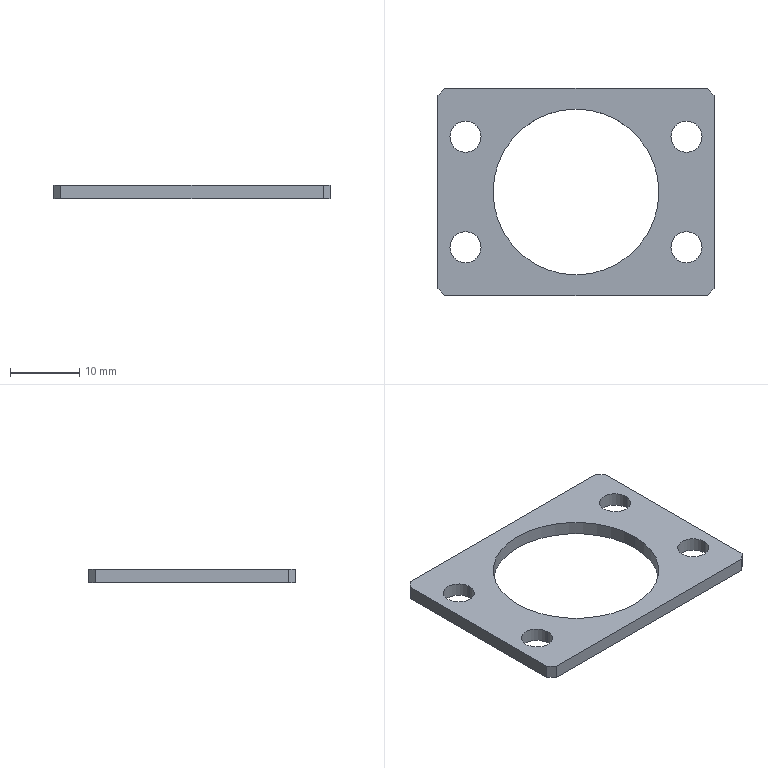Part | STEP file | Bearing stop plate | 1 solid | 20 faces | box 40 x 30 x 2 mm | volume 1364 mm3 | cylinder 10 | plane 10 | commonest cylinder face diameters 4.5 x8 24 x2
STEP:
#1=CARTESIAN_POINT('',(0.,0.,0.));
#2=DIRECTION('',(0.,0.,1.));
#3=DIRECTION('',(1.,0.,0.));
#4=AXIS2_PLACEMENT_3D('',#1,#2,#3);
#5=CARTESIAN_POINT('',(18.25,8.,-2.));
#6=VERTEX_POINT('',#5);
#7=CARTESIAN_POINT('',(18.25,8.,0.));
#8=VERTEX_POINT('',#7);
#9=CARTESIAN_POINT('',(18.25,8.,0.));
#10=DIRECTION('',(0.,0.,1.));
#11=VECTOR('',#10,1.);
#12=LINE('',#9,#11);
#13=CARTESIAN_POINT('',(16.,8.,0.));
#14=DIRECTION('',(0.,0.,1.));
#15=DIRECTION('',(1.,0.,0.));
#16=AXIS2_PLACEMENT_3D('',#13,#14,#15);
#17=CYLINDRICAL_SURFACE('',#16,2.25);
#18=CARTESIAN_POINT('',(6.283,0.));
#19=DIRECTION('',(0.,1.));
#20=VECTOR('',#19,1.);
#21=LINE('',#18,#20);
#22=(GEOMETRIC_REPRESENTATION_CONTEXT(2)PARAMETRIC_REPRESENTATION_CONTEXT()REPRESENTATION_CONTEXT('',''));
#23=DEFINITIONAL_REPRESENTATION('',(#21),#22);
#24=PCURVE('',#17,#23);
#25=CARTESIAN_POINT('',(16.,8.,0.));
#26=DIRECTION('',(0.,0.,1.));
#27=DIRECTION('',(1.,0.,0.));
#28=AXIS2_PLACEMENT_3D('',#25,#26,#27);
#29=CYLINDRICAL_SURFACE('',#28,2.25);
#30=CARTESIAN_POINT('',(0.,0.));
#31=DIRECTION('',(0.,1.));
#32=VECTOR('',#31,1.);
#33=LINE('',#30,#32);
#34=(GEOMETRIC_REPRESENTATION_CONTEXT(2)PARAMETRIC_REPRESENTATION_CONTEXT()REPRESENTATION_CONTEXT('',''));
#35=DEFINITIONAL_REPRESENTATION('',(#33),#34);
#36=PCURVE('',#29,#35);
#37=SURFACE_CURVE('',#12,(#24,#36),.PCURVE_S1.);
#38=EDGE_CURVE('',#6,#8,#37,.T.);
#39=ORIENTED_EDGE('',*,*,#38,.T.);
#40=CARTESIAN_POINT('',(13.75,8.,0.));
#41=VERTEX_POINT('',#40);
#42=CARTESIAN_POINT('',(16.,8.,0.));
#43=DIRECTION('',(0.,0.,1.));
#44=DIRECTION('',(1.,0.,0.));
#45=AXIS2_PLACEMENT_3D('',#42,#43,#44);
#46=CIRCLE('',#45,2.25);
#47=CARTESIAN_POINT('',(0.,0.));
#48=DIRECTION('',(1.,0.));
#49=VECTOR('',#48,1.);
#50=LINE('',#47,#49);
#51=(GEOMETRIC_REPRESENTATION_CONTEXT(2)PARAMETRIC_REPRESENTATION_CONTEXT()REPRESENTATION_CONTEXT('',''));
#52=DEFINITIONAL_REPRESENTATION('',(#50),#51);
#53=PCURVE('',#17,#52);
#54=CARTESIAN_POINT('',(20.,-15.,0.));
#55=DIRECTION('',(0.,0.,1.));
#56=DIRECTION('',(1.,0.,0.));
#57=AXIS2_PLACEMENT_3D('',#54,#55,#56);
#58=PLANE('',#57);
#59=CARTESIAN_POINT('',(-4.,23.));
#60=DIRECTION('',(1.,0.));
#61=AXIS2_PLACEMENT_2D('',#59,#60);
#62=CIRCLE('',#61,2.25);
#63=(GEOMETRIC_REPRESENTATION_CONTEXT(2)PARAMETRIC_REPRESENTATION_CONTEXT()REPRESENTATION_CONTEXT('',''));
#64=DEFINITIONAL_REPRESENTATION('',(#62),#63);
#65=PCURVE('',#58,#64);
#66=SURFACE_CURVE('',#46,(#53,#65),.PCURVE_S1.);
#67=EDGE_CURVE('',#41,#8,#66,.T.);
#68=ORIENTED_EDGE('',*,*,#67,.F.);
#69=CARTESIAN_POINT('',(13.75,8.,-2.));
#70=VERTEX_POINT('',#69);
#71=CARTESIAN_POINT('',(13.75,8.,0.));
#72=DIRECTION('',(0.,0.,1.));
#73=VECTOR('',#72,1.);
#74=LINE('',#71,#73);
#75=CARTESIAN_POINT('',(3.142,0.));
#76=DIRECTION('',(0.,1.));
#77=VECTOR('',#76,1.);
#78=LINE('',#75,#77);
#79=(GEOMETRIC_REPRESENTATION_CONTEXT(2)PARAMETRIC_REPRESENTATION_CONTEXT()REPRESENTATION_CONTEXT('',''));
#80=DEFINITIONAL_REPRESENTATION('',(#78),#79);
#81=PCURVE('',#17,#80);
#82=CARTESIAN_POINT('',(3.142,0.));
#83=DIRECTION('',(0.,1.));
#84=VECTOR('',#83,1.);
#85=LINE('',#82,#84);
#86=(GEOMETRIC_REPRESENTATION_CONTEXT(2)PARAMETRIC_REPRESENTATION_CONTEXT()REPRESENTATION_CONTEXT('',''));
#87=DEFINITIONAL_REPRESENTATION('',(#85),#86);
#88=PCURVE('',#29,#87);
#89=SURFACE_CURVE('',#74,(#81,#88),.PCURVE_S1.);
#90=EDGE_CURVE('',#70,#41,#89,.T.);
#91=ORIENTED_EDGE('',*,*,#90,.F.);
#92=CARTESIAN_POINT('',(16.,8.,-2.));
#93=DIRECTION('',(0.,0.,1.));
#94=DIRECTION('',(1.,0.,0.));
#95=AXIS2_PLACEMENT_3D('',#92,#93,#94);
#96=CIRCLE('',#95,2.25);
#97=CARTESIAN_POINT('',(0.,-2.));
#98=DIRECTION('',(1.,0.));
#99=VECTOR('',#98,1.);
#100=LINE('',#97,#99);
#101=(GEOMETRIC_REPRESENTATION_CONTEXT(2)PARAMETRIC_REPRESENTATION_CONTEXT()REPRESENTATION_CONTEXT('',''));
#102=DEFINITIONAL_REPRESENTATION('',(#100),#101);
#103=PCURVE('',#17,#102);
#104=CARTESIAN_POINT('',(20.,-15.,-2.));
#105=DIRECTION('',(0.,0.,1.));
#106=DIRECTION('',(1.,0.,0.));
#107=AXIS2_PLACEMENT_3D('',#104,#105,#106);
#108=PLANE('',#107);
#109=CARTESIAN_POINT('',(-4.,23.));
#110=DIRECTION('',(1.,0.));
#111=AXIS2_PLACEMENT_2D('',#109,#110);
#112=CIRCLE('',#111,2.25);
#113=(GEOMETRIC_REPRESENTATION_CONTEXT(2)PARAMETRIC_REPRESENTATION_CONTEXT()REPRESENTATION_CONTEXT('',''));
#114=DEFINITIONAL_REPRESENTATION('',(#112),#113);
#115=PCURVE('',#108,#114);
#116=SURFACE_CURVE('',#96,(#103,#115),.PCURVE_S1.);
#117=EDGE_CURVE('',#70,#6,#116,.T.);
#118=ORIENTED_EDGE('',*,*,#117,.T.);
#119=EDGE_LOOP('',(#39,#68,#91,#118));
#120=FACE_BOUND('',#119,.F.);
#121=ADVANCED_FACE('',(#120),#17,.F.);
#122=CARTESIAN_POINT('',(-13.75,8.,-2.));
#123=VERTEX_POINT('',#122);
#124=CARTESIAN_POINT('',(-13.75,8.,0.));
#125=VERTEX_POINT('',#124);
#126=CARTESIAN_POINT('',(-13.75,8.,0.));
#127=DIRECTION('',(0.,0.,1.));
#128=VECTOR('',#127,1.);
#129=LINE('',#126,#128);
#130=CARTESIAN_POINT('',(-16.,8.,0.));
#131=DIRECTION('',(0.,0.,1.));
#132=DIRECTION('',(1.,0.,0.));
#133=AXIS2_PLACEMENT_3D('',#130,#131,#132);
#134=CYLINDRICAL_SURFACE('',#133,2.25);
#135=CARTESIAN_POINT('',(6.283,0.));
#136=DIRECTION('',(0.,1.));
#137=VECTOR('',#136,1.);
#138=LINE('',#135,#137);
#139=(GEOMETRIC_REPRESENTATION_CONTEXT(2)PARAMETRIC_REPRESENTATION_CONTEXT()REPRESENTATION_CONTEXT('',''));
#140=DEFINITIONAL_REPRESENTATION('',(#138),#139);
#141=PCURVE('',#134,#140);
#142=CARTESIAN_POINT('',(-16.,8.,0.));
#143=DIRECTION('',(0.,0.,1.));
#144=DIRECTION('',(1.,0.,0.));
#145=AXIS2_PLACEMENT_3D('',#142,#143,#144);
#146=CYLINDRICAL_SURFACE('',#145,2.25);
#147=CARTESIAN_POINT('',(0.,0.));
#148=DIRECTION('',(0.,1.));
#149=VECTOR('',#148,1.);
#150=LINE('',#147,#149);
#151=(GEOMETRIC_REPRESENTATION_CONTEXT(2)PARAMETRIC_REPRESENTATION_CONTEXT()REPRESENTATION_CONTEXT('',''));
#152=DEFINITIONAL_REPRESENTATION('',(#150),#151);
#153=PCURVE('',#146,#152);
#154=SURFACE_CURVE('',#129,(#141,#153),.PCURVE_S1.);
#155=EDGE_CURVE('',#123,#125,#154,.T.);
#156=ORIENTED_EDGE('',*,*,#155,.T.);
#157=CARTESIAN_POINT('',(-18.25,8.,0.));
#158=VERTEX_POINT('',#157);
#159=CARTESIAN_POINT('',(-16.,8.,0.));
#160=DIRECTION('',(0.,0.,1.));
#161=DIRECTION('',(1.,0.,0.));
#162=AXIS2_PLACEMENT_3D('',#159,#160,#161);
#163=CIRCLE('',#162,2.25);
#164=CARTESIAN_POINT('',(0.,0.));
#165=DIRECTION('',(1.,0.));
#166=VECTOR('',#165,1.);
#167=LINE('',#164,#166);
#168=(GEOMETRIC_REPRESENTATION_CONTEXT(2)PARAMETRIC_REPRESENTATION_CONTEXT()REPRESENTATION_CONTEXT('',''));
#169=DEFINITIONAL_REPRESENTATION('',(#167),#168);
#170=PCURVE('',#134,#169);
#171=CARTESIAN_POINT('',(-36.,23.));
#172=DIRECTION('',(1.,0.));
#173=AXIS2_PLACEMENT_2D('',#171,#172);
#174=CIRCLE('',#173,2.25);
#175=(GEOMETRIC_REPRESENTATION_CONTEXT(2)PARAMETRIC_REPRESENTATION_CONTEXT()REPRESENTATION_CONTEXT('',''));
#176=DEFINITIONAL_REPRESENTATION('',(#174),#175);
#177=PCURVE('',#58,#176);
#178=SURFACE_CURVE('',#163,(#170,#177),.PCURVE_S1.);
#179=EDGE_CURVE('',#158,#125,#178,.T.);
#180=ORIENTED_EDGE('',*,*,#179,.F.);
#181=CARTESIAN_POINT('',(-18.25,8.,-2.));
#182=VERTEX_POINT('',#181);
#183=CARTESIAN_POINT('',(-18.25,8.,0.));
#184=DIRECTION('',(0.,0.,1.));
#185=VECTOR('',#184,1.);
#186=LINE('',#183,#185);
#187=CARTESIAN_POINT('',(3.142,0.));
#188=DIRECTION('',(0.,1.));
#189=VECTOR('',#188,1.);
#190=LINE('',#187,#189);
#191=(GEOMETRIC_REPRESENTATION_CONTEXT(2)PARAMETRIC_REPRESENTATION_CONTEXT()REPRESENTATION_CONTEXT('',''));
#192=DEFINITIONAL_REPRESENTATION('',(#190),#191);
#193=PCURVE('',#134,#192);
#194=CARTESIAN_POINT('',(3.142,0.));
#195=DIRECTION('',(0.,1.));
#196=VECTOR('',#195,1.);
#197=LINE('',#194,#196);
#198=(GEOMETRIC_REPRESENTATION_CONTEXT(2)PARAMETRIC_REPRESENTATION_CONTEXT()REPRESENTATION_CONTEXT('',''));
#199=DEFINITIONAL_REPRESENTATION('',(#197),#198);
#200=PCURVE('',#146,#199);
#201=SURFACE_CURVE('',#186,(#193,#200),.PCURVE_S1.);
#202=EDGE_CURVE('',#182,#158,#201,.T.);
#203=ORIENTED_EDGE('',*,*,#202,.F.);
#204=CARTESIAN_POINT('',(-16.,8.,-2.));
#205=DIRECTION('',(0.,0.,1.));
#206=DIRECTION('',(1.,0.,0.));
#207=AXIS2_PLACEMENT_3D('',#204,#205,#206);
#208=CIRCLE('',#207,2.25);
#209=CARTESIAN_POINT('',(0.,-2.));
#210=DIRECTION('',(1.,0.));
#211=VECTOR('',#210,1.);
#212=LINE('',#209,#211);
#213=(GEOMETRIC_REPRESENTATION_CONTEXT(2)PARAMETRIC_REPRESENTATION_CONTEXT()REPRESENTATION_CONTEXT('',''));
#214=DEFINITIONAL_REPRESENTATION('',(#212),#213);
#215=PCURVE('',#134,#214);
#216=CARTESIAN_POINT('',(-36.,23.));
#217=DIRECTION('',(1.,0.));
#218=AXIS2_PLACEMENT_2D('',#216,#217);
#219=CIRCLE('',#218,2.25);
#220=(GEOMETRIC_REPRESENTATION_CONTEXT(2)PARAMETRIC_REPRESENTATION_CONTEXT()REPRESENTATION_CONTEXT('',''));
#221=DEFINITIONAL_REPRESENTATION('',(#219),#220);
#222=PCURVE('',#108,#221);
#223=SURFACE_CURVE('',#208,(#215,#222),.PCURVE_S1.);
#224=EDGE_CURVE('',#182,#123,#223,.T.);
#225=ORIENTED_EDGE('',*,*,#224,.T.);
#226=EDGE_LOOP('',(#156,#180,#203,#225));
#227=FACE_BOUND('',#226,.F.);
#228=ADVANCED_FACE('',(#227),#134,.F.);
#229=CARTESIAN_POINT('',(-13.75,-8.,-2.));
#230=VERTEX_POINT('',#229);
#231=CARTESIAN_POINT('',(-13.75,-8.,0.));
#232=VERTEX_POINT('',#231);
#233=CARTESIAN_POINT('',(-13.75,-8.,0.));
#234=DIRECTION('',(0.,0.,1.));
#235=VECTOR('',#234,1.);
#236=LINE('',#233,#235);
#237=CARTESIAN_POINT('',(-16.,-8.,0.));
#238=DIRECTION('',(0.,0.,1.));
#239=DIRECTION('',(1.,0.,0.));
#240=AXIS2_PLACEMENT_3D('',#237,#238,#239);
#241=CYLINDRICAL_SURFACE('',#240,2.25);
#242=CARTESIAN_POINT('',(6.283,0.));
#243=DIRECTION('',(0.,1.));
#244=VECTOR('',#243,1.);
#245=LINE('',#242,#244);
#246=(GEOMETRIC_REPRESENTATION_CONTEXT(2)PARAMETRIC_REPRESENTATION_CONTEXT()REPRESENTATION_CONTEXT('',''));
#247=DEFINITIONAL_REPRESENTATION('',(#245),#246);
#248=PCURVE('',#241,#247);
#249=CARTESIAN_POINT('',(-16.,-8.,0.));
#250=DIRECTION('',(0.,0.,1.));
#251=DIRECTION('',(1.,0.,0.));
#252=AXIS2_PLACEMENT_3D('',#249,#250,#251);
#253=CYLINDRICAL_SURFACE('',#252,2.25);
#254=CARTESIAN_POINT('',(0.,0.));
#255=DIRECTION('',(0.,1.));
#256=VECTOR('',#255,1.);
#257=LINE('',#254,#256);
#258=(GEOMETRIC_REPRESENTATION_CONTEXT(2)PARAMETRIC_REPRESENTATION_CONTEXT()REPRESENTATION_CONTEXT('',''));
#259=DEFINITIONAL_REPRESENTATION('',(#257),#258);
#260=PCURVE('',#253,#259);
#261=SURFACE_CURVE('',#236,(#248,#260),.PCURVE_S1.);
#262=EDGE_CURVE('',#230,#232,#261,.T.);
#263=ORIENTED_EDGE('',*,*,#262,.T.);
#264=CARTESIAN_POINT('',(-18.25,-8.,0.));
#265=VERTEX_POINT('',#264);
#266=CARTESIAN_POINT('',(-16.,-8.,0.));
#267=DIRECTION('',(0.,0.,1.));
#268=DIRECTION('',(1.,0.,0.));
#269=AXIS2_PLACEMENT_3D('',#266,#267,#268);
#270=CIRCLE('',#269,2.25);
#271=CARTESIAN_POINT('',(0.,0.));
#272=DIRECTION('',(1.,0.));
#273=VECTOR('',#272,1.);
#274=LINE('',#271,#273);
#275=(GEOMETRIC_REPRESENTATION_CONTEXT(2)PARAMETRIC_REPRESENTATION_CONTEXT()REPRESENTATION_CONTEXT('',''));
#276=DEFINITIONAL_REPRESENTATION('',(#274),#275);
#277=PCURVE('',#241,#276);
#278=CARTESIAN_POINT('',(-36.,7.));
#279=DIRECTION('',(1.,0.));
#280=AXIS2_PLACEMENT_2D('',#278,#279);
#281=CIRCLE('',#280,2.25);
#282=(GEOMETRIC_REPRESENTATION_CONTEXT(2)PARAMETRIC_REPRESENTATION_CONTEXT()REPRESENTATION_CONTEXT('',''));
#283=DEFINITIONAL_REPRESENTATION('',(#281),#282);
#284=PCURVE('',#58,#283);
#285=SURFACE_CURVE('',#270,(#277,#284),.PCURVE_S1.);
#286=EDGE_CURVE('',#265,#232,#285,.T.);
#287=ORIENTED_EDGE('',*,*,#286,.F.);
#288=CARTESIAN_POINT('',(-18.25,-8.,-2.));
#289=VERTEX_POINT('',#288);
#290=CARTESIAN_POINT('',(-18.25,-8.,0.));
#291=DIRECTION('',(0.,0.,1.));
#292=VECTOR('',#291,1.);
#293=LINE('',#290,#292);
#294=CARTESIAN_POINT('',(3.142,0.));
#295=DIRECTION('',(0.,1.));
#296=VECTOR('',#295,1.);
#297=LINE('',#294,#296);
#298=(GEOMETRIC_REPRESENTATION_CONTEXT(2)PARAMETRIC_REPRESENTATION_CONTEXT()REPRESENTATION_CONTEXT('',''));
#299=DEFINITIONAL_REPRESENTATION('',(#297),#298);
#300=PCURVE('',#241,#299);
#301=CARTESIAN_POINT('',(3.142,0.));
#302=DIRECTION('',(0.,1.));
#303=VECTOR('',#302,1.);
#304=LINE('',#301,#303);
#305=(GEOMETRIC_REPRESENTATION_CONTEXT(2)PARAMETRIC_REPRESENTATION_CONTEXT()REPRESENTATION_CONTEXT('',''));
#306=DEFINITIONAL_REPRESENTATION('',(#304),#305);
#307=PCURVE('',#253,#306);
#308=SURFACE_CURVE('',#293,(#300,#307),.PCURVE_S1.);
#309=EDGE_CURVE('',#289,#265,#308,.T.);
#310=ORIENTED_EDGE('',*,*,#309,.F.);
#311=CARTESIAN_POINT('',(-16.,-8.,-2.));
#312=DIRECTION('',(0.,0.,1.));
#313=DIRECTION('',(1.,0.,0.));
#314=AXIS2_PLACEMENT_3D('',#311,#312,#313);
#315=CIRCLE('',#314,2.25);
#316=CARTESIAN_POINT('',(0.,-2.));
#317=DIRECTION('',(1.,0.));
#318=VECTOR('',#317,1.);
#319=LINE('',#316,#318);
#320=(GEOMETRIC_REPRESENTATION_CONTEXT(2)PARAMETRIC_REPRESENTATION_CONTEXT()REPRESENTATION_CONTEXT('',''));
#321=DEFINITIONAL_REPRESENTATION('',(#319),#320);
#322=PCURVE('',#241,#321);
#323=CARTESIAN_POINT('',(-36.,7.));
#324=DIRECTION('',(1.,0.));
#325=AXIS2_PLACEMENT_2D('',#323,#324);
#326=CIRCLE('',#325,2.25);
#327=(GEOMETRIC_REPRESENTATION_CONTEXT(2)PARAMETRIC_REPRESENTATION_CONTEXT()REPRESENTATION_CONTEXT('',''));
#328=DEFINITIONAL_REPRESENTATION('',(#326),#327);
#329=PCURVE('',#108,#328);
#330=SURFACE_CURVE('',#315,(#322,#329),.PCURVE_S1.);
#331=EDGE_CURVE('',#289,#230,#330,.T.);
#332=ORIENTED_EDGE('',*,*,#331,.T.);
#333=EDGE_LOOP('',(#263,#287,#310,#332));
#334=FACE_BOUND('',#333,.F.);
#335=ADVANCED_FACE('',(#334),#241,.F.);
#336=CARTESIAN_POINT('',(18.25,-8.,-2.));
#337=VERTEX_POINT('',#336);
#338=CARTESIAN_POINT('',(18.25,-8.,0.));
#339=VERTEX_POINT('',#338);
#340=CARTESIAN_POINT('',(18.25,-8.,0.));
#341=DIRECTION('',(0.,0.,1.));
#342=VECTOR('',#341,1.);
#343=LINE('',#340,#342);
#344=CARTESIAN_POINT('',(16.,-8.,0.));
#345=DIRECTION('',(0.,0.,1.));
#346=DIRECTION('',(1.,0.,0.));
#347=AXIS2_PLACEMENT_3D('',#344,#345,#346);
#348=CYLINDRICAL_SURFACE('',#347,2.25);
#349=CARTESIAN_POINT('',(6.283,0.));
#350=DIRECTION('',(0.,1.));
#351=VECTOR('',#350,1.);
#352=LINE('',#349,#351);
#353=(GEOMETRIC_REPRESENTATION_CONTEXT(2)PARAMETRIC_REPRESENTATION_CONTEXT()REPRESENTATION_CONTEXT('',''));
#354=DEFINITIONAL_REPRESENTATION('',(#352),#353);
#355=PCURVE('',#348,#354);
#356=CARTESIAN_POINT('',(16.,-8.,0.));
#357=DIRECTION('',(0.,0.,1.));
#358=DIRECTION('',(1.,0.,0.));
#359=AXIS2_PLACEMENT_3D('',#356,#357,#358);
#360=CYLINDRICAL_SURFACE('',#359,2.25);
#361=CARTESIAN_POINT('',(0.,0.));
#362=DIRECTION('',(0.,1.));
#363=VECTOR('',#362,1.);
#364=LINE('',#361,#363);
#365=(GEOMETRIC_REPRESENTATION_CONTEXT(2)PARAMETRIC_REPRESENTATION_CONTEXT()REPRESENTATION_CONTEXT('',''));
#366=DEFINITIONAL_REPRESENTATION('',(#364),#365);
#367=PCURVE('',#360,#366);
#368=SURFACE_CURVE('',#343,(#355,#367),.PCURVE_S1.);
#369=EDGE_CURVE('',#337,#339,#368,.T.);
#370=ORIENTED_EDGE('',*,*,#369,.T.);
#371=CARTESIAN_POINT('',(13.75,-8.,0.));
#372=VERTEX_POINT('',#371);
#373=CARTESIAN_POINT('',(16.,-8.,0.));
#374=DIRECTION('',(0.,0.,1.));
#375=DIRECTION('',(1.,0.,0.));
#376=AXIS2_PLACEMENT_3D('',#373,#374,#375);
#377=CIRCLE('',#376,2.25);
#378=CARTESIAN_POINT('',(0.,0.));
#379=DIRECTION('',(1.,0.));
#380=VECTOR('',#379,1.);
#381=LINE('',#378,#380);
#382=(GEOMETRIC_REPRESENTATION_CONTEXT(2)PARAMETRIC_REPRESENTATION_CONTEXT()REPRESENTATION_CONTEXT('',''));
#383=DEFINITIONAL_REPRESENTATION('',(#381),#382);
#384=PCURVE('',#348,#383);
#385=CARTESIAN_POINT('',(-4.,7.));
#386=DIRECTION('',(1.,0.));
#387=AXIS2_PLACEMENT_2D('',#385,#386);
#388=CIRCLE('',#387,2.25);
#389=(GEOMETRIC_REPRESENTATION_CONTEXT(2)PARAMETRIC_REPRESENTATION_CONTEXT()REPRESENTATION_CONTEXT('',''));
#390=DEFINITIONAL_REPRESENTATION('',(#388),#389);
#391=PCURVE('',#58,#390);
#392=SURFACE_CURVE('',#377,(#384,#391),.PCURVE_S1.);
#393=EDGE_CURVE('',#372,#339,#392,.T.);
#394=ORIENTED_EDGE('',*,*,#393,.F.);
#395=CARTESIAN_POINT('',(13.75,-8.,-2.));
#396=VERTEX_POINT('',#395);
#397=CARTESIAN_POINT('',(13.75,-8.,0.));
#398=DIRECTION('',(0.,0.,1.));
#399=VECTOR('',#398,1.);
#400=LINE('',#397,#399);
#401=CARTESIAN_POINT('',(3.142,0.));
#402=DIRECTION('',(0.,1.));
#403=VECTOR('',#402,1.);
#404=LINE('',#401,#403);
#405=(GEOMETRIC_REPRESENTATION_CONTEXT(2)PARAMETRIC_REPRESENTATION_CONTEXT()REPRESENTATION_CONTEXT('',''));
#406=DEFINITIONAL_REPRESENTATION('',(#404),#405);
#407=PCURVE('',#348,#406);
#408=CARTESIAN_POINT('',(3.142,0.));
#409=DIRECTION('',(0.,1.));
#410=VECTOR('',#409,1.);
#411=LINE('',#408,#410);
#412=(GEOMETRIC_REPRESENTATION_CONTEXT(2)PARAMETRIC_REPRESENTATION_CONTEXT()REPRESENTATION_CONTEXT('',''));
#413=DEFINITIONAL_REPRESENTATION('',(#411),#412);
#414=PCURVE('',#360,#413);
#415=SURFACE_CURVE('',#400,(#407,#414),.PCURVE_S1.);
#416=EDGE_CURVE('',#396,#372,#415,.T.);
#417=ORIENTED_EDGE('',*,*,#416,.F.);
#418=CARTESIAN_POINT('',(16.,-8.,-2.));
#419=DIRECTION('',(0.,0.,1.));
#420=DIRECTION('',(1.,0.,0.));
#421=AXIS2_PLACEMENT_3D('',#418,#419,#420);
#422=CIRCLE('',#421,2.25);
#423=CARTESIAN_POINT('',(0.,-2.));
#424=DIRECTION('',(1.,0.));
#425=VECTOR('',#424,1.);
#426=LINE('',#423,#425);
#427=(GEOMETRIC_REPRESENTATION_CONTEXT(2)PARAMETRIC_REPRESENTATION_CONTEXT()REPRESENTATION_CONTEXT('',''));
#428=DEFINITIONAL_REPRESENTATION('',(#426),#427);
#429=PCURVE('',#348,#428);
#430=CARTESIAN_POINT('',(-4.,7.));
#431=DIRECTION('',(1.,0.));
#432=AXIS2_PLACEMENT_2D('',#430,#431);
#433=CIRCLE('',#432,2.25);
#434=(GEOMETRIC_REPRESENTATION_CONTEXT(2)PARAMETRIC_REPRESENTATION_CONTEXT()REPRESENTATION_CONTEXT('',''));
#435=DEFINITIONAL_REPRESENTATION('',(#433),#434);
#436=PCURVE('',#108,#435);
#437=SURFACE_CURVE('',#422,(#429,#436),.PCURVE_S1.);
#438=EDGE_CURVE('',#396,#337,#437,.T.);
#439=ORIENTED_EDGE('',*,*,#438,.T.);
#440=EDGE_LOOP('',(#370,#394,#417,#439));
#441=FACE_BOUND('',#440,.F.);
#442=ADVANCED_FACE('',(#441),#348,.F.);
#443=CARTESIAN_POINT('',(12.,0.,-2.));
#444=VERTEX_POINT('',#443);
#445=CARTESIAN_POINT('',(12.,0.,0.));
#446=VERTEX_POINT('',#445);
#447=CARTESIAN_POINT('',(12.,0.,-2.));
#448=DIRECTION('',(0.,0.,1.));
#449=VECTOR('',#448,1.);
#450=LINE('',#447,#449);
#451=CARTESIAN_POINT('',(0.,0.,-2.));
#452=DIRECTION('',(0.,0.,1.));
#453=DIRECTION('',(1.,0.,0.));
#454=AXIS2_PLACEMENT_3D('',#451,#452,#453);
#455=CYLINDRICAL_SURFACE('',#454,12.);
#456=CARTESIAN_POINT('',(6.283,0.));
#457=DIRECTION('',(0.,1.));
#458=VECTOR('',#457,1.);
#459=LINE('',#456,#458);
#460=(GEOMETRIC_REPRESENTATION_CONTEXT(2)PARAMETRIC_REPRESENTATION_CONTEXT()REPRESENTATION_CONTEXT('',''));
#461=DEFINITIONAL_REPRESENTATION('',(#459),#460);
#462=PCURVE('',#455,#461);
#463=CARTESIAN_POINT('',(0.,0.,-2.));
#464=DIRECTION('',(0.,0.,1.));
#465=DIRECTION('',(1.,0.,0.));
#466=AXIS2_PLACEMENT_3D('',#463,#464,#465);
#467=CYLINDRICAL_SURFACE('',#466,12.);
#468=CARTESIAN_POINT('',(0.,0.));
#469=DIRECTION('',(0.,1.));
#470=VECTOR('',#469,1.);
#471=LINE('',#468,#470);
#472=(GEOMETRIC_REPRESENTATION_CONTEXT(2)PARAMETRIC_REPRESENTATION_CONTEXT()REPRESENTATION_CONTEXT('',''));
#473=DEFINITIONAL_REPRESENTATION('',(#471),#472);
#474=PCURVE('',#467,#473);
#475=SURFACE_CURVE('',#450,(#462,#474),.PCURVE_S1.);
#476=EDGE_CURVE('',#444,#446,#475,.T.);
#477=ORIENTED_EDGE('',*,*,#476,.T.);
#478=CARTESIAN_POINT('',(-12.,0.,0.));
#479=VERTEX_POINT('',#478);
#480=CARTESIAN_POINT('',(0.,0.,0.));
#481=DIRECTION('',(0.,0.,1.));
#482=DIRECTION('',(1.,0.,0.));
#483=AXIS2_PLACEMENT_3D('',#480,#481,#482);
#484=CIRCLE('',#483,12.);
#485=CARTESIAN_POINT('',(0.,2.));
#486=DIRECTION('',(1.,0.));
#487=VECTOR('',#486,1.);
#488=LINE('',#485,#487);
#489=(GEOMETRIC_REPRESENTATION_CONTEXT(2)PARAMETRIC_REPRESENTATION_CONTEXT()REPRESENTATION_CONTEXT('',''));
#490=DEFINITIONAL_REPRESENTATION('',(#488),#489);
#491=PCURVE('',#455,#490);
#492=CARTESIAN_POINT('',(-20.,15.));
#493=DIRECTION('',(1.,0.));
#494=AXIS2_PLACEMENT_2D('',#492,#493);
#495=CIRCLE('',#494,12.);
#496=(GEOMETRIC_REPRESENTATION_CONTEXT(2)PARAMETRIC_REPRESENTATION_CONTEXT()REPRESENTATION_CONTEXT('',''));
#497=DEFINITIONAL_REPRESENTATION('',(#495),#496);
#498=PCURVE('',#58,#497);
#499=SURFACE_CURVE('',#484,(#491,#498),.PCURVE_S1.);
#500=EDGE_CURVE('',#479,#446,#499,.T.);
#501=ORIENTED_EDGE('',*,*,#500,.F.);
#502=CARTESIAN_POINT('',(-12.,0.,-2.));
#503=VERTEX_POINT('',#502);
#504=CARTESIAN_POINT('',(-12.,0.,-2.));
#505=DIRECTION('',(0.,0.,1.));
#506=VECTOR('',#505,1.);
#507=LINE('',#504,#506);
#508=CARTESIAN_POINT('',(3.142,0.));
#509=DIRECTION('',(0.,1.));
#510=VECTOR('',#509,1.);
#511=LINE('',#508,#510);
#512=(GEOMETRIC_REPRESENTATION_CONTEXT(2)PARAMETRIC_REPRESENTATION_CONTEXT()REPRESENTATION_CONTEXT('',''));
#513=DEFINITIONAL_REPRESENTATION('',(#511),#512);
#514=PCURVE('',#455,#513);
#515=CARTESIAN_POINT('',(3.142,0.));
#516=DIRECTION('',(0.,1.));
#517=VECTOR('',#516,1.);
#518=LINE('',#515,#517);
#519=(GEOMETRIC_REPRESENTATION_CONTEXT(2)PARAMETRIC_REPRESENTATION_CONTEXT()REPRESENTATION_CONTEXT('',''));
#520=DEFINITIONAL_REPRESENTATION('',(#518),#519);
#521=PCURVE('',#467,#520);
#522=SURFACE_CURVE('',#507,(#514,#521),.PCURVE_S1.);
#523=EDGE_CURVE('',#503,#479,#522,.T.);
#524=ORIENTED_EDGE('',*,*,#523,.F.);
#525=CARTESIAN_POINT('',(0.,0.,-2.));
#526=DIRECTION('',(0.,0.,1.));
#527=DIRECTION('',(1.,0.,0.));
#528=AXIS2_PLACEMENT_3D('',#525,#526,#527);
#529=CIRCLE('',#528,12.);
#530=CARTESIAN_POINT('',(0.,0.));
#531=DIRECTION('',(1.,0.));
#532=VECTOR('',#531,1.);
#533=LINE('',#530,#532);
#534=(GEOMETRIC_REPRESENTATION_CONTEXT(2)PARAMETRIC_REPRESENTATION_CONTEXT()REPRESENTATION_CONTEXT('',''));
#535=DEFINITIONAL_REPRESENTATION('',(#533),#534);
#536=PCURVE('',#455,#535);
#537=CARTESIAN_POINT('',(-20.,15.));
#538=DIRECTION('',(1.,0.));
#539=AXIS2_PLACEMENT_2D('',#537,#538);
#540=CIRCLE('',#539,12.);
#541=(GEOMETRIC_REPRESENTATION_CONTEXT(2)PARAMETRIC_REPRESENTATION_CONTEXT()REPRESENTATION_CONTEXT('',''));
#542=DEFINITIONAL_REPRESENTATION('',(#540),#541);
#543=PCURVE('',#108,#542);
#544=SURFACE_CURVE('',#529,(#536,#543),.PCURVE_S1.);
#545=EDGE_CURVE('',#503,#444,#544,.T.);
#546=ORIENTED_EDGE('',*,*,#545,.T.);
#547=EDGE_LOOP('',(#477,#501,#524,#546));
#548=FACE_BOUND('',#547,.F.);
#549=ADVANCED_FACE('',(#548),#455,.F.);
#550=CARTESIAN_POINT('',(20.,-14.,0.));
#551=VERTEX_POINT('',#550);
#552=CARTESIAN_POINT('',(20.,14.,0.));
#553=VERTEX_POINT('',#552);
#554=CARTESIAN_POINT('',(20.,15.,0.));
#555=DIRECTION('',(0.,1.,0.));
#556=VECTOR('',#555,1.);
#557=LINE('',#554,#556);
#558=CARTESIAN_POINT('',(20.,15.,-2.));
#559=DIRECTION('',(1.,0.,0.));
#560=DIRECTION('',(0.,1.,0.));
#561=AXIS2_PLACEMENT_3D('',#558,#559,#560);
#562=PLANE('',#561);
#563=CARTESIAN_POINT('',(0.,2.));
#564=DIRECTION('',(1.,0.));
#565=VECTOR('',#564,1.);
#566=LINE('',#563,#565);
#567=(GEOMETRIC_REPRESENTATION_CONTEXT(2)PARAMETRIC_REPRESENTATION_CONTEXT()REPRESENTATION_CONTEXT('',''));
#568=DEFINITIONAL_REPRESENTATION('',(#566),#567);
#569=PCURVE('',#562,#568);
#570=CARTESIAN_POINT('',(0.,30.));
#571=DIRECTION('',(0.,1.));
#572=VECTOR('',#571,1.);
#573=LINE('',#570,#572);
#574=(GEOMETRIC_REPRESENTATION_CONTEXT(2)PARAMETRIC_REPRESENTATION_CONTEXT()REPRESENTATION_CONTEXT('',''));
#575=DEFINITIONAL_REPRESENTATION('',(#573),#574);
#576=PCURVE('',#58,#575);
#577=SURFACE_CURVE('',#557,(#569,#576),.PCURVE_S1.);
#578=EDGE_CURVE('',#551,#553,#577,.T.);
#579=ORIENTED_EDGE('',*,*,#578,.F.);
#580=CARTESIAN_POINT('',(20.,-14.,-2.));
#581=VERTEX_POINT('',#580);
#582=CARTESIAN_POINT('',(20.,-14.,-2.));
#583=DIRECTION('',(0.,0.,-1.));
#584=VECTOR('',#583,1.);
#585=LINE('',#582,#584);
#586=CARTESIAN_POINT('',(-29.,0.));
#587=DIRECTION('',(0.,-1.));
#588=VECTOR('',#587,1.);
#589=LINE('',#586,#588);
#590=(GEOMETRIC_REPRESENTATION_CONTEXT(2)PARAMETRIC_REPRESENTATION_CONTEXT()REPRESENTATION_CONTEXT('',''));
#591=DEFINITIONAL_REPRESENTATION('',(#589),#590);
#592=PCURVE('',#562,#591);
#593=CARTESIAN_POINT('',(19.,-15.,-2.));
#594=DIRECTION('',(-0.7071,0.7071,0.));
#595=DIRECTION('',(-0.7071,-0.7071,0.));
#596=AXIS2_PLACEMENT_3D('',#593,#594,#595);
#597=PLANE('',#596);
#598=CARTESIAN_POINT('',(-1.414,0.));
#599=DIRECTION('',(0.,-1.));
#600=VECTOR('',#599,1.);
#601=LINE('',#598,#600);
#602=(GEOMETRIC_REPRESENTATION_CONTEXT(2)PARAMETRIC_REPRESENTATION_CONTEXT()REPRESENTATION_CONTEXT('',''));
#603=DEFINITIONAL_REPRESENTATION('',(#601),#602);
#604=PCURVE('',#597,#603);
#605=SURFACE_CURVE('',#585,(#592,#604),.PCURVE_S1.);
#606=EDGE_CURVE('',#551,#581,#605,.T.);
#607=ORIENTED_EDGE('',*,*,#606,.T.);
#608=CARTESIAN_POINT('',(20.,14.,-2.));
#609=VERTEX_POINT('',#608);
#610=CARTESIAN_POINT('',(20.,15.,-2.));
#611=DIRECTION('',(0.,1.,0.));
#612=VECTOR('',#611,1.);
#613=LINE('',#610,#612);
#614=CARTESIAN_POINT('',(0.,0.));
#615=DIRECTION('',(1.,0.));
#616=VECTOR('',#615,1.);
#617=LINE('',#614,#616);
#618=(GEOMETRIC_REPRESENTATION_CONTEXT(2)PARAMETRIC_REPRESENTATION_CONTEXT()REPRESENTATION_CONTEXT('',''));
#619=DEFINITIONAL_REPRESENTATION('',(#617),#618);
#620=PCURVE('',#562,#619);
#621=CARTESIAN_POINT('',(0.,30.));
#622=DIRECTION('',(0.,1.));
#623=VECTOR('',#622,1.);
#624=LINE('',#621,#623);
#625=(GEOMETRIC_REPRESENTATION_CONTEXT(2)PARAMETRIC_REPRESENTATION_CONTEXT()REPRESENTATION_CONTEXT('',''));
#626=DEFINITIONAL_REPRESENTATION('',(#624),#625);
#627=PCURVE('',#108,#626);
#628=SURFACE_CURVE('',#613,(#620,#627),.PCURVE_S1.);
#629=EDGE_CURVE('',#581,#609,#628,.T.);
#630=ORIENTED_EDGE('',*,*,#629,.T.);
#631=CARTESIAN_POINT('',(20.,14.,-2.));
#632=DIRECTION('',(0.,0.,1.));
#633=VECTOR('',#632,1.);
#634=LINE('',#631,#633);
#635=CARTESIAN_POINT('',(-1.,0.));
#636=DIRECTION('',(0.,1.));
#637=VECTOR('',#636,1.);
#638=LINE('',#635,#637);
#639=(GEOMETRIC_REPRESENTATION_CONTEXT(2)PARAMETRIC_REPRESENTATION_CONTEXT()REPRESENTATION_CONTEXT('',''));
#640=DEFINITIONAL_REPRESENTATION('',(#638),#639);
#641=PCURVE('',#562,#640);
#642=CARTESIAN_POINT('',(20.,14.,-2.));
#643=DIRECTION('',(-0.7071,-0.7071,0.));
#644=DIRECTION('',(0.7071,-0.7071,0.));
#645=AXIS2_PLACEMENT_3D('',#642,#643,#644);
#646=PLANE('',#645);
#647=CARTESIAN_POINT('',(0.,0.));
#648=DIRECTION('',(0.,1.));
#649=VECTOR('',#648,1.);
#650=LINE('',#647,#649);
#651=(GEOMETRIC_REPRESENTATION_CONTEXT(2)PARAMETRIC_REPRESENTATION_CONTEXT()REPRESENTATION_CONTEXT('',''));
#652=DEFINITIONAL_REPRESENTATION('',(#650),#651);
#653=PCURVE('',#646,#652);
#654=SURFACE_CURVE('',#634,(#641,#653),.PCURVE_S1.);
#655=EDGE_CURVE('',#609,#553,#654,.T.);
#656=ORIENTED_EDGE('',*,*,#655,.T.);
#657=EDGE_LOOP('',(#579,#607,#630,#656));
#658=FACE_BOUND('',#657,.T.);
#659=ADVANCED_FACE('',(#658),#562,.T.);
#660=CARTESIAN_POINT('',(-19.,-15.,-2.));
#661=VERTEX_POINT('',#660);
#662=CARTESIAN_POINT('',(19.,-15.,-2.));
#663=VERTEX_POINT('',#662);
#664=CARTESIAN_POINT('',(-20.,-15.,-2.));
#665=DIRECTION('',(1.,0.,0.));
#666=VECTOR('',#665,1.);
#667=LINE('',#664,#666);
#668=CARTESIAN_POINT('',(-20.,-15.,-2.));
#669=DIRECTION('',(0.,-1.,0.));
#670=DIRECTION('',(0.,0.,-1.));
#671=AXIS2_PLACEMENT_3D('',#668,#669,#670);
#672=PLANE('',#671);
#673=CARTESIAN_POINT('',(0.,0.));
#674=DIRECTION('',(0.,1.));
#675=VECTOR('',#674,1.);
#676=LINE('',#673,#675);
#677=(GEOMETRIC_REPRESENTATION_CONTEXT(2)PARAMETRIC_REPRESENTATION_CONTEXT()REPRESENTATION_CONTEXT('',''));
#678=DEFINITIONAL_REPRESENTATION('',(#676),#677);
#679=PCURVE('',#672,#678);
#680=CARTESIAN_POINT('',(-40.,0.));
#681=DIRECTION('',(1.,0.));
#682=VECTOR('',#681,1.);
#683=LINE('',#680,#682);
#684=(GEOMETRIC_REPRESENTATION_CONTEXT(2)PARAMETRIC_REPRESENTATION_CONTEXT()REPRESENTATION_CONTEXT('',''));
#685=DEFINITIONAL_REPRESENTATION('',(#683),#684);
#686=PCURVE('',#108,#685);
#687=SURFACE_CURVE('',#667,(#679,#686),.PCURVE_S1.);
#688=EDGE_CURVE('',#661,#663,#687,.T.);
#689=ORIENTED_EDGE('',*,*,#688,.T.);
#690=CARTESIAN_POINT('',(19.,-15.,0.));
#691=VERTEX_POINT('',#690);
#692=CARTESIAN_POINT('',(19.,-15.,-2.));
#693=DIRECTION('',(0.,0.,1.));
#694=VECTOR('',#693,1.);
#695=LINE('',#692,#694);
#696=CARTESIAN_POINT('',(0.,39.));
#697=DIRECTION('',(-1.,0.));
#698=VECTOR('',#697,1.);
#699=LINE('',#696,#698);
#700=(GEOMETRIC_REPRESENTATION_CONTEXT(2)PARAMETRIC_REPRESENTATION_CONTEXT()REPRESENTATION_CONTEXT('',''));
#701=DEFINITIONAL_REPRESENTATION('',(#699),#700);
#702=PCURVE('',#672,#701);
#703=CARTESIAN_POINT('',(0.,0.));
#704=DIRECTION('',(0.,1.));
#705=VECTOR('',#704,1.);
#706=LINE('',#703,#705);
#707=(GEOMETRIC_REPRESENTATION_CONTEXT(2)PARAMETRIC_REPRESENTATION_CONTEXT()REPRESENTATION_CONTEXT('',''));
#708=DEFINITIONAL_REPRESENTATION('',(#706),#707);
#709=PCURVE('',#597,#708);
#710=SURFACE_CURVE('',#695,(#702,#709),.PCURVE_S1.);
#711=EDGE_CURVE('',#663,#691,#710,.T.);
#712=ORIENTED_EDGE('',*,*,#711,.T.);
#713=CARTESIAN_POINT('',(-19.,-15.,0.));
#714=VERTEX_POINT('',#713);
#715=CARTESIAN_POINT('',(-20.,-15.,0.));
#716=DIRECTION('',(1.,0.,0.));
#717=VECTOR('',#716,1.);
#718=LINE('',#715,#717);
#719=CARTESIAN_POINT('',(-2.,0.));
#720=DIRECTION('',(0.,1.));
#721=VECTOR('',#720,1.);
#722=LINE('',#719,#721);
#723=(GEOMETRIC_REPRESENTATION_CONTEXT(2)PARAMETRIC_REPRESENTATION_CONTEXT()REPRESENTATION_CONTEXT('',''));
#724=DEFINITIONAL_REPRESENTATION('',(#722),#723);
#725=PCURVE('',#672,#724);
#726=CARTESIAN_POINT('',(-40.,0.));
#727=DIRECTION('',(1.,0.));
#728=VECTOR('',#727,1.);
#729=LINE('',#726,#728);
#730=(GEOMETRIC_REPRESENTATION_CONTEXT(2)PARAMETRIC_REPRESENTATION_CONTEXT()REPRESENTATION_CONTEXT('',''));
#731=DEFINITIONAL_REPRESENTATION('',(#729),#730);
#732=PCURVE('',#58,#731);
#733=SURFACE_CURVE('',#718,(#725,#732),.PCURVE_S1.);
#734=EDGE_CURVE('',#714,#691,#733,.T.);
#735=ORIENTED_EDGE('',*,*,#734,.F.);
#736=CARTESIAN_POINT('',(-19.,-15.,-2.));
#737=DIRECTION('',(0.,0.,-1.));
#738=VECTOR('',#737,1.);
#739=LINE('',#736,#738);
#740=CARTESIAN_POINT('',(0.,1.));
#741=DIRECTION('',(1.,0.));
#742=VECTOR('',#741,1.);
#743=LINE('',#740,#742);
#744=(GEOMETRIC_REPRESENTATION_CONTEXT(2)PARAMETRIC_REPRESENTATION_CONTEXT()REPRESENTATION_CONTEXT('',''));
#745=DEFINITIONAL_REPRESENTATION('',(#743),#744);
#746=PCURVE('',#672,#745);
#747=CARTESIAN_POINT('',(-20.,-14.,-2.));
#748=DIRECTION('',(0.7071,0.7071,0.));
#749=DIRECTION('',(-0.7071,0.7071,0.));
#750=AXIS2_PLACEMENT_3D('',#747,#748,#749);
#751=PLANE('',#750);
#752=CARTESIAN_POINT('',(-1.414,0.));
#753=DIRECTION('',(0.,-1.));
#754=VECTOR('',#753,1.);
#755=LINE('',#752,#754);
#756=(GEOMETRIC_REPRESENTATION_CONTEXT(2)PARAMETRIC_REPRESENTATION_CONTEXT()REPRESENTATION_CONTEXT('',''));
#757=DEFINITIONAL_REPRESENTATION('',(#755),#756);
#758=PCURVE('',#751,#757);
#759=SURFACE_CURVE('',#739,(#746,#758),.PCURVE_S1.);
#760=EDGE_CURVE('',#714,#661,#759,.T.);
#761=ORIENTED_EDGE('',*,*,#760,.T.);
#762=EDGE_LOOP('',(#689,#712,#735,#761));
#763=FACE_BOUND('',#762,.T.);
#764=ADVANCED_FACE('',(#763),#672,.T.);
#765=CARTESIAN_POINT('',(-20.,14.,-2.));
#766=VERTEX_POINT('',#765);
#767=CARTESIAN_POINT('',(-20.,-14.,-2.));
#768=VERTEX_POINT('',#767);
#769=CARTESIAN_POINT('',(-20.,15.,-2.));
#770=DIRECTION('',(0.,-1.,0.));
#771=VECTOR('',#770,1.);
#772=LINE('',#769,#771);
#773=CARTESIAN_POINT('',(-20.,15.,-2.));
#774=DIRECTION('',(-1.,0.,0.));
#775=DIRECTION('',(0.,-1.,0.));
#776=AXIS2_PLACEMENT_3D('',#773,#774,#775);
#777=PLANE('',#776);
#778=CARTESIAN_POINT('',(0.,0.));
#779=DIRECTION('',(1.,0.));
#780=VECTOR('',#779,1.);
#781=LINE('',#778,#780);
#782=(GEOMETRIC_REPRESENTATION_CONTEXT(2)PARAMETRIC_REPRESENTATION_CONTEXT()REPRESENTATION_CONTEXT('',''));
#783=DEFINITIONAL_REPRESENTATION('',(#781),#782);
#784=PCURVE('',#777,#783);
#785=CARTESIAN_POINT('',(-40.,30.));
#786=DIRECTION('',(0.,-1.));
#787=VECTOR('',#786,1.);
#788=LINE('',#785,#787);
#789=(GEOMETRIC_REPRESENTATION_CONTEXT(2)PARAMETRIC_REPRESENTATION_CONTEXT()REPRESENTATION_CONTEXT('',''));
#790=DEFINITIONAL_REPRESENTATION('',(#788),#789);
#791=PCURVE('',#108,#790);
#792=SURFACE_CURVE('',#772,(#784,#791),.PCURVE_S1.);
#793=EDGE_CURVE('',#766,#768,#792,.T.);
#794=ORIENTED_EDGE('',*,*,#793,.T.);
#795=CARTESIAN_POINT('',(-20.,-14.,0.));
#796=VERTEX_POINT('',#795);
#797=CARTESIAN_POINT('',(-20.,-14.,-2.));
#798=DIRECTION('',(0.,0.,1.));
#799=VECTOR('',#798,1.);
#800=LINE('',#797,#799);
#801=CARTESIAN_POINT('',(29.,0.));
#802=DIRECTION('',(0.,1.));
#803=VECTOR('',#802,1.);
#804=LINE('',#801,#803);
#805=(GEOMETRIC_REPRESENTATION_CONTEXT(2)PARAMETRIC_REPRESENTATION_CONTEXT()REPRESENTATION_CONTEXT('',''));
#806=DEFINITIONAL_REPRESENTATION('',(#804),#805);
#807=PCURVE('',#777,#806);
#808=CARTESIAN_POINT('',(0.,0.));
#809=DIRECTION('',(0.,1.));
#810=VECTOR('',#809,1.);
#811=LINE('',#808,#810);
#812=(GEOMETRIC_REPRESENTATION_CONTEXT(2)PARAMETRIC_REPRESENTATION_CONTEXT()REPRESENTATION_CONTEXT('',''));
#813=DEFINITIONAL_REPRESENTATION('',(#811),#812);
#814=PCURVE('',#751,#813);
#815=SURFACE_CURVE('',#800,(#807,#814),.PCURVE_S1.);
#816=EDGE_CURVE('',#768,#796,#815,.T.);
#817=ORIENTED_EDGE('',*,*,#816,.T.);
#818=CARTESIAN_POINT('',(-20.,14.,0.));
#819=VERTEX_POINT('',#818);
#820=CARTESIAN_POINT('',(-20.,15.,0.));
#821=DIRECTION('',(0.,-1.,0.));
#822=VECTOR('',#821,1.);
#823=LINE('',#820,#822);
#824=CARTESIAN_POINT('',(0.,2.));
#825=DIRECTION('',(1.,0.));
#826=VECTOR('',#825,1.);
#827=LINE('',#824,#826);
#828=(GEOMETRIC_REPRESENTATION_CONTEXT(2)PARAMETRIC_REPRESENTATION_CONTEXT()REPRESENTATION_CONTEXT('',''));
#829=DEFINITIONAL_REPRESENTATION('',(#827),#828);
#830=PCURVE('',#777,#829);
#831=CARTESIAN_POINT('',(-40.,30.));
#832=DIRECTION('',(0.,-1.));
#833=VECTOR('',#832,1.);
#834=LINE('',#831,#833);
#835=(GEOMETRIC_REPRESENTATION_CONTEXT(2)PARAMETRIC_REPRESENTATION_CONTEXT()REPRESENTATION_CONTEXT('',''));
#836=DEFINITIONAL_REPRESENTATION('',(#834),#835);
#837=PCURVE('',#58,#836);
#838=SURFACE_CURVE('',#823,(#830,#837),.PCURVE_S1.);
#839=EDGE_CURVE('',#819,#796,#838,.T.);
#840=ORIENTED_EDGE('',*,*,#839,.F.);
#841=CARTESIAN_POINT('',(-20.,14.,-2.));
#842=DIRECTION('',(0.,0.,-1.));
#843=VECTOR('',#842,1.);
#844=LINE('',#841,#843);
#845=CARTESIAN_POINT('',(1.,0.));
#846=DIRECTION('',(0.,-1.));
#847=VECTOR('',#846,1.);
#848=LINE('',#845,#847);
#849=(GEOMETRIC_REPRESENTATION_CONTEXT(2)PARAMETRIC_REPRESENTATION_CONTEXT()REPRESENTATION_CONTEXT('',''));
#850=DEFINITIONAL_REPRESENTATION('',(#848),#849);
#851=PCURVE('',#777,#850);
#852=CARTESIAN_POINT('',(-19.,15.,-2.));
#853=DIRECTION('',(0.7071,-0.7071,0.));
#854=DIRECTION('',(0.7071,0.7071,0.));
#855=AXIS2_PLACEMENT_3D('',#852,#853,#854);
#856=PLANE('',#855);
#857=CARTESIAN_POINT('',(-1.414,0.));
#858=DIRECTION('',(0.,-1.));
#859=VECTOR('',#858,1.);
#860=LINE('',#857,#859);
#861=(GEOMETRIC_REPRESENTATION_CONTEXT(2)PARAMETRIC_REPRESENTATION_CONTEXT()REPRESENTATION_CONTEXT('',''));
#862=DEFINITIONAL_REPRESENTATION('',(#860),#861);
#863=PCURVE('',#856,#862);
#864=SURFACE_CURVE('',#844,(#851,#863),.PCURVE_S1.);
#865=EDGE_CURVE('',#819,#766,#864,.T.);
#866=ORIENTED_EDGE('',*,*,#865,.T.);
#867=EDGE_LOOP('',(#794,#817,#840,#866));
#868=FACE_BOUND('',#867,.T.);
#869=ADVANCED_FACE('',(#868),#777,.T.);
#870=CARTESIAN_POINT('',(19.,15.,0.));
#871=VERTEX_POINT('',#870);
#872=CARTESIAN_POINT('',(-19.,15.,0.));
#873=VERTEX_POINT('',#872);
#874=CARTESIAN_POINT('',(-20.,15.,0.));
#875=DIRECTION('',(-1.,0.,0.));
#876=VECTOR('',#875,1.);
#877=LINE('',#874,#876);
#878=CARTESIAN_POINT('',(-20.,15.,-2.));
#879=DIRECTION('',(0.,1.,0.));
#880=DIRECTION('',(0.,0.,1.));
#881=AXIS2_PLACEMENT_3D('',#878,#879,#880);
#882=PLANE('',#881);
#883=CARTESIAN_POINT('',(2.,0.));
#884=DIRECTION('',(0.,-1.));
#885=VECTOR('',#884,1.);
#886=LINE('',#883,#885);
#887=(GEOMETRIC_REPRESENTATION_CONTEXT(2)PARAMETRIC_REPRESENTATION_CONTEXT()REPRESENTATION_CONTEXT('',''));
#888=DEFINITIONAL_REPRESENTATION('',(#886),#887);
#889=PCURVE('',#882,#888);
#890=CARTESIAN_POINT('',(-40.,30.));
#891=DIRECTION('',(-1.,0.));
#892=VECTOR('',#891,1.);
#893=LINE('',#890,#892);
#894=(GEOMETRIC_REPRESENTATION_CONTEXT(2)PARAMETRIC_REPRESENTATION_CONTEXT()REPRESENTATION_CONTEXT('',''));
#895=DEFINITIONAL_REPRESENTATION('',(#893),#894);
#896=PCURVE('',#58,#895);
#897=SURFACE_CURVE('',#877,(#889,#896),.PCURVE_S1.);
#898=EDGE_CURVE('',#871,#873,#897,.T.);
#899=ORIENTED_EDGE('',*,*,#898,.F.);
#900=CARTESIAN_POINT('',(19.,15.,-2.));
#901=VERTEX_POINT('',#900);
#902=CARTESIAN_POINT('',(19.,15.,-2.));
#903=DIRECTION('',(0.,0.,-1.));
#904=VECTOR('',#903,1.);
#905=LINE('',#902,#904);
#906=CARTESIAN_POINT('',(0.,39.));
#907=DIRECTION('',(-1.,0.));
#908=VECTOR('',#907,1.);
#909=LINE('',#906,#908);
#910=(GEOMETRIC_REPRESENTATION_CONTEXT(2)PARAMETRIC_REPRESENTATION_CONTEXT()REPRESENTATION_CONTEXT('',''));
#911=DEFINITIONAL_REPRESENTATION('',(#909),#910);
#912=PCURVE('',#882,#911);
#913=CARTESIAN_POINT('',(-1.414,0.));
#914=DIRECTION('',(0.,-1.));
#915=VECTOR('',#914,1.);
#916=LINE('',#913,#915);
#917=(GEOMETRIC_REPRESENTATION_CONTEXT(2)PARAMETRIC_REPRESENTATION_CONTEXT()REPRESENTATION_CONTEXT('',''));
#918=DEFINITIONAL_REPRESENTATION('',(#916),#917);
#919=PCURVE('',#646,#918);
#920=SURFACE_CURVE('',#905,(#912,#919),.PCURVE_S1.);
#921=EDGE_CURVE('',#871,#901,#920,.T.);
#922=ORIENTED_EDGE('',*,*,#921,.T.);
#923=CARTESIAN_POINT('',(-19.,15.,-2.));
#924=VERTEX_POINT('',#923);
#925=CARTESIAN_POINT('',(-20.,15.,-2.));
#926=DIRECTION('',(-1.,0.,0.));
#927=VECTOR('',#926,1.);
#928=LINE('',#925,#927);
#929=CARTESIAN_POINT('',(0.,0.));
#930=DIRECTION('',(0.,-1.));
#931=VECTOR('',#930,1.);
#932=LINE('',#929,#931);
#933=(GEOMETRIC_REPRESENTATION_CONTEXT(2)PARAMETRIC_REPRESENTATION_CONTEXT()REPRESENTATION_CONTEXT('',''));
#934=DEFINITIONAL_REPRESENTATION('',(#932),#933);
#935=PCURVE('',#882,#934);
#936=CARTESIAN_POINT('',(-40.,30.));
#937=DIRECTION('',(-1.,0.));
#938=VECTOR('',#937,1.);
#939=LINE('',#936,#938);
#940=(GEOMETRIC_REPRESENTATION_CONTEXT(2)PARAMETRIC_REPRESENTATION_CONTEXT()REPRESENTATION_CONTEXT('',''));
#941=DEFINITIONAL_REPRESENTATION('',(#939),#940);
#942=PCURVE('',#108,#941);
#943=SURFACE_CURVE('',#928,(#935,#942),.PCURVE_S1.);
#944=EDGE_CURVE('',#901,#924,#943,.T.);
#945=ORIENTED_EDGE('',*,*,#944,.T.);
#946=CARTESIAN_POINT('',(-19.,15.,-2.));
#947=DIRECTION('',(0.,0.,1.));
#948=VECTOR('',#947,1.);
#949=LINE('',#946,#948);
#950=CARTESIAN_POINT('',(0.,1.));
#951=DIRECTION('',(1.,0.));
#952=VECTOR('',#951,1.);
#953=LINE('',#950,#952);
#954=(GEOMETRIC_REPRESENTATION_CONTEXT(2)PARAMETRIC_REPRESENTATION_CONTEXT()REPRESENTATION_CONTEXT('',''));
#955=DEFINITIONAL_REPRESENTATION('',(#953),#954);
#956=PCURVE('',#882,#955);
#957=CARTESIAN_POINT('',(0.,0.));
#958=DIRECTION('',(0.,1.));
#959=VECTOR('',#958,1.);
#960=LINE('',#957,#959);
#961=(GEOMETRIC_REPRESENTATION_CONTEXT(2)PARAMETRIC_REPRESENTATION_CONTEXT()REPRESENTATION_CONTEXT('',''));
#962=DEFINITIONAL_REPRESENTATION('',(#960),#961);
#963=PCURVE('',#856,#962);
#964=SURFACE_CURVE('',#949,(#956,#963),.PCURVE_S1.);
#965=EDGE_CURVE('',#924,#873,#964,.T.);
#966=ORIENTED_EDGE('',*,*,#965,.T.);
#967=EDGE_LOOP('',(#899,#922,#945,#966));
#968=FACE_BOUND('',#967,.T.);
#969=ADVANCED_FACE('',(#968),#882,.T.);
#970=CARTESIAN_POINT('',(16.,8.,-2.));
#971=DIRECTION('',(0.,0.,1.));
#972=DIRECTION('',(1.,0.,0.));
#973=AXIS2_PLACEMENT_3D('',#970,#971,#972);
#974=CIRCLE('',#973,2.25);
#975=CARTESIAN_POINT('',(-4.,23.));
#976=DIRECTION('',(1.,0.));
#977=AXIS2_PLACEMENT_2D('',#975,#976);
#978=CIRCLE('',#977,2.25);
#979=(GEOMETRIC_REPRESENTATION_CONTEXT(2)PARAMETRIC_REPRESENTATION_CONTEXT()REPRESENTATION_CONTEXT('',''));
#980=DEFINITIONAL_REPRESENTATION('',(#978),#979);
#981=PCURVE('',#108,#980);
#982=CARTESIAN_POINT('',(0.,-2.));
#983=DIRECTION('',(1.,0.));
#984=VECTOR('',#983,1.);
#985=LINE('',#982,#984);
#986=(GEOMETRIC_REPRESENTATION_CONTEXT(2)PARAMETRIC_REPRESENTATION_CONTEXT()REPRESENTATION_CONTEXT('',''));
#987=DEFINITIONAL_REPRESENTATION('',(#985),#986);
#988=PCURVE('',#29,#987);
#989=SURFACE_CURVE('',#974,(#981,#988),.PCURVE_S1.);
#990=EDGE_CURVE('',#6,#70,#989,.T.);
#991=ORIENTED_EDGE('',*,*,#990,.T.);
#992=ORIENTED_EDGE('',*,*,#117,.T.);
#993=EDGE_LOOP('',(#991,#992));
#994=FACE_BOUND('',#993,.T.);
#995=CARTESIAN_POINT('',(-16.,8.,-2.));
#996=DIRECTION('',(0.,0.,1.));
#997=DIRECTION('',(1.,0.,0.));
#998=AXIS2_PLACEMENT_3D('',#995,#996,#997);
#999=CIRCLE('',#998,2.25);
#1000=CARTESIAN_POINT('',(-36.,23.));
#1001=DIRECTION('',(1.,0.));
#1002=AXIS2_PLACEMENT_2D('',#1000,#1001);
#1003=CIRCLE('',#1002,2.25);
#1004=(GEOMETRIC_REPRESENTATION_CONTEXT(2)PARAMETRIC_REPRESENTATION_CONTEXT()REPRESENTATION_CONTEXT('',''));
#1005=DEFINITIONAL_REPRESENTATION('',(#1003),#1004);
#1006=PCURVE('',#108,#1005);
#1007=CARTESIAN_POINT('',(0.,-2.));
#1008=DIRECTION('',(1.,0.));
#1009=VECTOR('',#1008,1.);
#1010=LINE('',#1007,#1009);
#1011=(GEOMETRIC_REPRESENTATION_CONTEXT(2)PARAMETRIC_REPRESENTATION_CONTEXT()REPRESENTATION_CONTEXT('',''));
#1012=DEFINITIONAL_REPRESENTATION('',(#1010),#1011);
#1013=PCURVE('',#146,#1012);
#1014=SURFACE_CURVE('',#999,(#1006,#1013),.PCURVE_S1.);
#1015=EDGE_CURVE('',#123,#182,#1014,.T.);
#1016=ORIENTED_EDGE('',*,*,#1015,.T.);
#1017=ORIENTED_EDGE('',*,*,#224,.T.);
#1018=EDGE_LOOP('',(#1016,#1017));
#1019=FACE_BOUND('',#1018,.T.);
#1020=CARTESIAN_POINT('',(-16.,-8.,-2.));
#1021=DIRECTION('',(0.,0.,1.));
#1022=DIRECTION('',(1.,0.,0.));
#1023=AXIS2_PLACEMENT_3D('',#1020,#1021,#1022);
#1024=CIRCLE('',#1023,2.25);
#1025=CARTESIAN_POINT('',(-36.,7.));
#1026=DIRECTION('',(1.,0.));
#1027=AXIS2_PLACEMENT_2D('',#1025,#1026);
#1028=CIRCLE('',#1027,2.25);
#1029=(GEOMETRIC_REPRESENTATION_CONTEXT(2)PARAMETRIC_REPRESENTATION_CONTEXT()REPRESENTATION_CONTEXT('',''));
#1030=DEFINITIONAL_REPRESENTATION('',(#1028),#1029);
#1031=PCURVE('',#108,#1030);
#1032=CARTESIAN_POINT('',(0.,-2.));
#1033=DIRECTION('',(1.,0.));
#1034=VECTOR('',#1033,1.);
#1035=LINE('',#1032,#1034);
#1036=(GEOMETRIC_REPRESENTATION_CONTEXT(2)PARAMETRIC_REPRESENTATION_CONTEXT()REPRESENTATION_CONTEXT('',''));
#1037=DEFINITIONAL_REPRESENTATION('',(#1035),#1036);
#1038=PCURVE('',#253,#1037);
#1039=SURFACE_CURVE('',#1024,(#1031,#1038),.PCURVE_S1.);
#1040=EDGE_CURVE('',#230,#289,#1039,.T.);
#1041=ORIENTED_EDGE('',*,*,#1040,.T.);
#1042=ORIENTED_EDGE('',*,*,#331,.T.);
#1043=EDGE_LOOP('',(#1041,#1042));
#1044=FACE_BOUND('',#1043,.T.);
#1045=CARTESIAN_POINT('',(16.,-8.,-2.));
#1046=DIRECTION('',(0.,0.,1.));
#1047=DIRECTION('',(1.,0.,0.));
#1048=AXIS2_PLACEMENT_3D('',#1045,#1046,#1047);
#1049=CIRCLE('',#1048,2.25);
#1050=CARTESIAN_POINT('',(-4.,7.));
#1051=DIRECTION('',(1.,0.));
#1052=AXIS2_PLACEMENT_2D('',#1050,#1051);
#1053=CIRCLE('',#1052,2.25);
#1054=(GEOMETRIC_REPRESENTATION_CONTEXT(2)PARAMETRIC_REPRESENTATION_CONTEXT()REPRESENTATION_CONTEXT('',''));
#1055=DEFINITIONAL_REPRESENTATION('',(#1053),#1054);
#1056=PCURVE('',#108,#1055);
#1057=CARTESIAN_POINT('',(0.,-2.));
#1058=DIRECTION('',(1.,0.));
#1059=VECTOR('',#1058,1.);
#1060=LINE('',#1057,#1059);
#1061=(GEOMETRIC_REPRESENTATION_CONTEXT(2)PARAMETRIC_REPRESENTATION_CONTEXT()REPRESENTATION_CONTEXT('',''));
#1062=DEFINITIONAL_REPRESENTATION('',(#1060),#1061);
#1063=PCURVE('',#360,#1062);
#1064=SURFACE_CURVE('',#1049,(#1056,#1063),.PCURVE_S1.);
#1065=EDGE_CURVE('',#337,#396,#1064,.T.);
#1066=ORIENTED_EDGE('',*,*,#1065,.T.);
#1067=ORIENTED_EDGE('',*,*,#438,.T.);
#1068=EDGE_LOOP('',(#1066,#1067));
#1069=FACE_BOUND('',#1068,.T.);
#1070=CARTESIAN_POINT('',(0.,0.,-2.));
#1071=DIRECTION('',(0.,0.,1.));
#1072=DIRECTION('',(1.,0.,0.));
#1073=AXIS2_PLACEMENT_3D('',#1070,#1071,#1072);
#1074=CIRCLE('',#1073,12.);
#1075=CARTESIAN_POINT('',(-20.,15.));
#1076=DIRECTION('',(1.,0.));
#1077=AXIS2_PLACEMENT_2D('',#1075,#1076);
#1078=CIRCLE('',#1077,12.);
#1079=(GEOMETRIC_REPRESENTATION_CONTEXT(2)PARAMETRIC_REPRESENTATION_CONTEXT()REPRESENTATION_CONTEXT('',''));
#1080=DEFINITIONAL_REPRESENTATION('',(#1078),#1079);
#1081=PCURVE('',#108,#1080);
#1082=CARTESIAN_POINT('',(0.,0.));
#1083=DIRECTION('',(1.,0.));
#1084=VECTOR('',#1083,1.);
#1085=LINE('',#1082,#1084);
#1086=(GEOMETRIC_REPRESENTATION_CONTEXT(2)PARAMETRIC_REPRESENTATION_CONTEXT()REPRESENTATION_CONTEXT('',''));
#1087=DEFINITIONAL_REPRESENTATION('',(#1085),#1086);
#1088=PCURVE('',#467,#1087);
#1089=SURFACE_CURVE('',#1074,(#1081,#1088),.PCURVE_S1.);
#1090=EDGE_CURVE('',#444,#503,#1089,.T.);
#1091=ORIENTED_EDGE('',*,*,#1090,.T.);
#1092=ORIENTED_EDGE('',*,*,#545,.T.);
#1093=EDGE_LOOP('',(#1091,#1092));
#1094=FACE_BOUND('',#1093,.T.);
#1095=ORIENTED_EDGE('',*,*,#629,.F.);
#1096=CARTESIAN_POINT('',(19.,-15.,-2.));
#1097=DIRECTION('',(-0.7071,-0.7071,0.));
#1098=VECTOR('',#1097,1.);
#1099=LINE('',#1096,#1098);
#1100=CARTESIAN_POINT('',(-1.,0.));
#1101=DIRECTION('',(-0.7071,-0.7071));
#1102=VECTOR('',#1101,1.);
#1103=LINE('',#1100,#1102);
#1104=(GEOMETRIC_REPRESENTATION_CONTEXT(2)PARAMETRIC_REPRESENTATION_CONTEXT()REPRESENTATION_CONTEXT('',''));
#1105=DEFINITIONAL_REPRESENTATION('',(#1103),#1104);
#1106=PCURVE('',#108,#1105);
#1107=CARTESIAN_POINT('',(0.,0.));
#1108=DIRECTION('',(1.,0.));
#1109=VECTOR('',#1108,1.);
#1110=LINE('',#1107,#1109);
#1111=(GEOMETRIC_REPRESENTATION_CONTEXT(2)PARAMETRIC_REPRESENTATION_CONTEXT()REPRESENTATION_CONTEXT('',''));
#1112=DEFINITIONAL_REPRESENTATION('',(#1110),#1111);
#1113=PCURVE('',#597,#1112);
#1114=SURFACE_CURVE('',#1099,(#1106,#1113),.PCURVE_S1.);
#1115=EDGE_CURVE('',#581,#663,#1114,.T.);
#1116=ORIENTED_EDGE('',*,*,#1115,.T.);
#1117=ORIENTED_EDGE('',*,*,#688,.F.);
#1118=CARTESIAN_POINT('',(-20.,-14.,-2.));
#1119=DIRECTION('',(-0.7071,0.7071,0.));
#1120=VECTOR('',#1119,1.);
#1121=LINE('',#1118,#1120);
#1122=CARTESIAN_POINT('',(-40.,1.));
#1123=DIRECTION('',(-0.7071,0.7071));
#1124=VECTOR('',#1123,1.);
#1125=LINE('',#1122,#1124);
#1126=(GEOMETRIC_REPRESENTATION_CONTEXT(2)PARAMETRIC_REPRESENTATION_CONTEXT()REPRESENTATION_CONTEXT('',''));
#1127=DEFINITIONAL_REPRESENTATION('',(#1125),#1126);
#1128=PCURVE('',#108,#1127);
#1129=CARTESIAN_POINT('',(0.,0.));
#1130=DIRECTION('',(1.,0.));
#1131=VECTOR('',#1130,1.);
#1132=LINE('',#1129,#1131);
#1133=(GEOMETRIC_REPRESENTATION_CONTEXT(2)PARAMETRIC_REPRESENTATION_CONTEXT()REPRESENTATION_CONTEXT('',''));
#1134=DEFINITIONAL_REPRESENTATION('',(#1132),#1133);
#1135=PCURVE('',#751,#1134);
#1136=SURFACE_CURVE('',#1121,(#1128,#1135),.PCURVE_S1.);
#1137=EDGE_CURVE('',#661,#768,#1136,.T.);
#1138=ORIENTED_EDGE('',*,*,#1137,.T.);
#1139=ORIENTED_EDGE('',*,*,#793,.F.);
#1140=CARTESIAN_POINT('',(-19.,15.,-2.));
#1141=DIRECTION('',(0.7071,0.7071,0.));
#1142=VECTOR('',#1141,1.);
#1143=LINE('',#1140,#1142);
#1144=CARTESIAN_POINT('',(-39.,30.));
#1145=DIRECTION('',(0.7071,0.7071));
#1146=VECTOR('',#1145,1.);
#1147=LINE('',#1144,#1146);
#1148=(GEOMETRIC_REPRESENTATION_CONTEXT(2)PARAMETRIC_REPRESENTATION_CONTEXT()REPRESENTATION_CONTEXT('',''));
#1149=DEFINITIONAL_REPRESENTATION('',(#1147),#1148);
#1150=PCURVE('',#108,#1149);
#1151=CARTESIAN_POINT('',(0.,0.));
#1152=DIRECTION('',(1.,0.));
#1153=VECTOR('',#1152,1.);
#1154=LINE('',#1151,#1153);
#1155=(GEOMETRIC_REPRESENTATION_CONTEXT(2)PARAMETRIC_REPRESENTATION_CONTEXT()REPRESENTATION_CONTEXT('',''));
#1156=DEFINITIONAL_REPRESENTATION('',(#1154),#1155);
#1157=PCURVE('',#856,#1156);
#1158=SURFACE_CURVE('',#1143,(#1150,#1157),.PCURVE_S1.);
#1159=EDGE_CURVE('',#766,#924,#1158,.T.);
#1160=ORIENTED_EDGE('',*,*,#1159,.T.);
#1161=ORIENTED_EDGE('',*,*,#944,.F.);
#1162=CARTESIAN_POINT('',(20.,14.,-2.));
#1163=DIRECTION('',(0.7071,-0.7071,0.));
#1164=VECTOR('',#1163,1.);
#1165=LINE('',#1162,#1164);
#1166=CARTESIAN_POINT('',(0.,29.));
#1167=DIRECTION('',(0.7071,-0.7071));
#1168=VECTOR('',#1167,1.);
#1169=LINE('',#1166,#1168);
#1170=(GEOMETRIC_REPRESENTATION_CONTEXT(2)PARAMETRIC_REPRESENTATION_CONTEXT()REPRESENTATION_CONTEXT('',''));
#1171=DEFINITIONAL_REPRESENTATION('',(#1169),#1170);
#1172=PCURVE('',#108,#1171);
#1173=CARTESIAN_POINT('',(0.,0.));
#1174=DIRECTION('',(1.,0.));
#1175=VECTOR('',#1174,1.);
#1176=LINE('',#1173,#1175);
#1177=(GEOMETRIC_REPRESENTATION_CONTEXT(2)PARAMETRIC_REPRESENTATION_CONTEXT()REPRESENTATION_CONTEXT('',''));
#1178=DEFINITIONAL_REPRESENTATION('',(#1176),#1177);
#1179=PCURVE('',#646,#1178);
#1180=SURFACE_CURVE('',#1165,(#1172,#1179),.PCURVE_S1.);
#1181=EDGE_CURVE('',#901,#609,#1180,.T.);
#1182=ORIENTED_EDGE('',*,*,#1181,.T.);
#1183=EDGE_LOOP('',(#1095,#1116,#1117,#1138,#1139,#1160,#1161,#1182));
#1184=FACE_BOUND('',#1183,.T.);
#1185=ADVANCED_FACE('',(#994,#1019,#1044,#1069,#1094,#1184),#108,.F.);
#1186=CARTESIAN_POINT('',(16.,8.,0.));
#1187=DIRECTION('',(0.,0.,1.));
#1188=DIRECTION('',(1.,0.,0.));
#1189=AXIS2_PLACEMENT_3D('',#1186,#1187,#1188);
#1190=CIRCLE('',#1189,2.25);
#1191=CARTESIAN_POINT('',(-4.,23.));
#1192=DIRECTION('',(1.,0.));
#1193=AXIS2_PLACEMENT_2D('',#1191,#1192);
#1194=CIRCLE('',#1193,2.25);
#1195=(GEOMETRIC_REPRESENTATION_CONTEXT(2)PARAMETRIC_REPRESENTATION_CONTEXT()REPRESENTATION_CONTEXT('',''));
#1196=DEFINITIONAL_REPRESENTATION('',(#1194),#1195);
#1197=PCURVE('',#58,#1196);
#1198=CARTESIAN_POINT('',(0.,0.));
#1199=DIRECTION('',(1.,0.));
#1200=VECTOR('',#1199,1.);
#1201=LINE('',#1198,#1200);
#1202=(GEOMETRIC_REPRESENTATION_CONTEXT(2)PARAMETRIC_REPRESENTATION_CONTEXT()REPRESENTATION_CONTEXT('',''));
#1203=DEFINITIONAL_REPRESENTATION('',(#1201),#1202);
#1204=PCURVE('',#29,#1203);
#1205=SURFACE_CURVE('',#1190,(#1197,#1204),.PCURVE_S1.);
#1206=EDGE_CURVE('',#8,#41,#1205,.T.);
#1207=ORIENTED_EDGE('',*,*,#1206,.F.);
#1208=ORIENTED_EDGE('',*,*,#67,.F.);
#1209=EDGE_LOOP('',(#1207,#1208));
#1210=FACE_BOUND('',#1209,.T.);
#1211=CARTESIAN_POINT('',(-16.,8.,0.));
#1212=DIRECTION('',(0.,0.,1.));
#1213=DIRECTION('',(1.,0.,0.));
#1214=AXIS2_PLACEMENT_3D('',#1211,#1212,#1213);
#1215=CIRCLE('',#1214,2.25);
#1216=CARTESIAN_POINT('',(-36.,23.));
#1217=DIRECTION('',(1.,0.));
#1218=AXIS2_PLACEMENT_2D('',#1216,#1217);
#1219=CIRCLE('',#1218,2.25);
#1220=(GEOMETRIC_REPRESENTATION_CONTEXT(2)PARAMETRIC_REPRESENTATION_CONTEXT()REPRESENTATION_CONTEXT('',''));
#1221=DEFINITIONAL_REPRESENTATION('',(#1219),#1220);
#1222=PCURVE('',#58,#1221);
#1223=CARTESIAN_POINT('',(0.,0.));
#1224=DIRECTION('',(1.,0.));
#1225=VECTOR('',#1224,1.);
#1226=LINE('',#1223,#1225);
#1227=(GEOMETRIC_REPRESENTATION_CONTEXT(2)PARAMETRIC_REPRESENTATION_CONTEXT()REPRESENTATION_CONTEXT('',''));
#1228=DEFINITIONAL_REPRESENTATION('',(#1226),#1227);
#1229=PCURVE('',#146,#1228);
#1230=SURFACE_CURVE('',#1215,(#1222,#1229),.PCURVE_S1.);
#1231=EDGE_CURVE('',#125,#158,#1230,.T.);
#1232=ORIENTED_EDGE('',*,*,#1231,.F.);
#1233=ORIENTED_EDGE('',*,*,#179,.F.);
#1234=EDGE_LOOP('',(#1232,#1233));
#1235=FACE_BOUND('',#1234,.T.);
#1236=CARTESIAN_POINT('',(-16.,-8.,0.));
#1237=DIRECTION('',(0.,0.,1.));
#1238=DIRECTION('',(1.,0.,0.));
#1239=AXIS2_PLACEMENT_3D('',#1236,#1237,#1238);
#1240=CIRCLE('',#1239,2.25);
#1241=CARTESIAN_POINT('',(-36.,7.));
#1242=DIRECTION('',(1.,0.));
#1243=AXIS2_PLACEMENT_2D('',#1241,#1242);
#1244=CIRCLE('',#1243,2.25);
#1245=(GEOMETRIC_REPRESENTATION_CONTEXT(2)PARAMETRIC_REPRESENTATION_CONTEXT()REPRESENTATION_CONTEXT('',''));
#1246=DEFINITIONAL_REPRESENTATION('',(#1244),#1245);
#1247=PCURVE('',#58,#1246);
#1248=CARTESIAN_POINT('',(0.,0.));
#1249=DIRECTION('',(1.,0.));
#1250=VECTOR('',#1249,1.);
#1251=LINE('',#1248,#1250);
#1252=(GEOMETRIC_REPRESENTATION_CONTEXT(2)PARAMETRIC_REPRESENTATION_CONTEXT()REPRESENTATION_CONTEXT('',''));
#1253=DEFINITIONAL_REPRESENTATION('',(#1251),#1252);
#1254=PCURVE('',#253,#1253);
#1255=SURFACE_CURVE('',#1240,(#1247,#1254),.PCURVE_S1.);
#1256=EDGE_CURVE('',#232,#265,#1255,.T.);
#1257=ORIENTED_EDGE('',*,*,#1256,.F.);
#1258=ORIENTED_EDGE('',*,*,#286,.F.);
#1259=EDGE_LOOP('',(#1257,#1258));
#1260=FACE_BOUND('',#1259,.T.);
#1261=CARTESIAN_POINT('',(16.,-8.,0.));
#1262=DIRECTION('',(0.,0.,1.));
#1263=DIRECTION('',(1.,0.,0.));
#1264=AXIS2_PLACEMENT_3D('',#1261,#1262,#1263);
#1265=CIRCLE('',#1264,2.25);
#1266=CARTESIAN_POINT('',(-4.,7.));
#1267=DIRECTION('',(1.,0.));
#1268=AXIS2_PLACEMENT_2D('',#1266,#1267);
#1269=CIRCLE('',#1268,2.25);
#1270=(GEOMETRIC_REPRESENTATION_CONTEXT(2)PARAMETRIC_REPRESENTATION_CONTEXT()REPRESENTATION_CONTEXT('',''));
#1271=DEFINITIONAL_REPRESENTATION('',(#1269),#1270);
#1272=PCURVE('',#58,#1271);
#1273=CARTESIAN_POINT('',(0.,0.));
#1274=DIRECTION('',(1.,0.));
#1275=VECTOR('',#1274,1.);
#1276=LINE('',#1273,#1275);
#1277=(GEOMETRIC_REPRESENTATION_CONTEXT(2)PARAMETRIC_REPRESENTATION_CONTEXT()REPRESENTATION_CONTEXT('',''));
#1278=DEFINITIONAL_REPRESENTATION('',(#1276),#1277);
#1279=PCURVE('',#360,#1278);
#1280=SURFACE_CURVE('',#1265,(#1272,#1279),.PCURVE_S1.);
#1281=EDGE_CURVE('',#339,#372,#1280,.T.);
#1282=ORIENTED_EDGE('',*,*,#1281,.F.);
#1283=ORIENTED_EDGE('',*,*,#393,.F.);
#1284=EDGE_LOOP('',(#1282,#1283));
#1285=FACE_BOUND('',#1284,.T.);
#1286=CARTESIAN_POINT('',(0.,0.,0.));
#1287=DIRECTION('',(0.,0.,1.));
#1288=DIRECTION('',(1.,0.,0.));
#1289=AXIS2_PLACEMENT_3D('',#1286,#1287,#1288);
#1290=CIRCLE('',#1289,12.);
#1291=CARTESIAN_POINT('',(-20.,15.));
#1292=DIRECTION('',(1.,0.));
#1293=AXIS2_PLACEMENT_2D('',#1291,#1292);
#1294=CIRCLE('',#1293,12.);
#1295=(GEOMETRIC_REPRESENTATION_CONTEXT(2)PARAMETRIC_REPRESENTATION_CONTEXT()REPRESENTATION_CONTEXT('',''));
#1296=DEFINITIONAL_REPRESENTATION('',(#1294),#1295);
#1297=PCURVE('',#58,#1296);
#1298=CARTESIAN_POINT('',(0.,2.));
#1299=DIRECTION('',(1.,0.));
#1300=VECTOR('',#1299,1.);
#1301=LINE('',#1298,#1300);
#1302=(GEOMETRIC_REPRESENTATION_CONTEXT(2)PARAMETRIC_REPRESENTATION_CONTEXT()REPRESENTATION_CONTEXT('',''));
#1303=DEFINITIONAL_REPRESENTATION('',(#1301),#1302);
#1304=PCURVE('',#467,#1303);
#1305=SURFACE_CURVE('',#1290,(#1297,#1304),.PCURVE_S1.);
#1306=EDGE_CURVE('',#446,#479,#1305,.T.);
#1307=ORIENTED_EDGE('',*,*,#1306,.F.);
#1308=ORIENTED_EDGE('',*,*,#500,.F.);
#1309=EDGE_LOOP('',(#1307,#1308));
#1310=FACE_BOUND('',#1309,.T.);
#1311=ORIENTED_EDGE('',*,*,#734,.T.);
#1312=CARTESIAN_POINT('',(19.5,-14.5,0.));
#1313=DIRECTION('',(0.7071,0.7071,0.));
#1314=VECTOR('',#1313,1.);
#1315=LINE('',#1312,#1314);
#1316=CARTESIAN_POINT('',(-0.5,0.5));
#1317=DIRECTION('',(0.7071,0.7071));
#1318=VECTOR('',#1317,1.);
#1319=LINE('',#1316,#1318);
#1320=(GEOMETRIC_REPRESENTATION_CONTEXT(2)PARAMETRIC_REPRESENTATION_CONTEXT()REPRESENTATION_CONTEXT('',''));
#1321=DEFINITIONAL_REPRESENTATION('',(#1319),#1320);
#1322=PCURVE('',#58,#1321);
#1323=CARTESIAN_POINT('',(-0.7071,2.));
#1324=DIRECTION('',(-1.,0.));
#1325=VECTOR('',#1324,1.);
#1326=LINE('',#1323,#1325);
#1327=(GEOMETRIC_REPRESENTATION_CONTEXT(2)PARAMETRIC_REPRESENTATION_CONTEXT()REPRESENTATION_CONTEXT('',''));
#1328=DEFINITIONAL_REPRESENTATION('',(#1326),#1327);
#1329=PCURVE('',#597,#1328);
#1330=SURFACE_CURVE('',#1315,(#1322,#1329),.PCURVE_S1.);
#1331=EDGE_CURVE('',#691,#551,#1330,.T.);
#1332=ORIENTED_EDGE('',*,*,#1331,.T.);
#1333=ORIENTED_EDGE('',*,*,#578,.T.);
#1334=CARTESIAN_POINT('',(34.5,-0.5,0.));
#1335=DIRECTION('',(-0.7071,0.7071,0.));
#1336=VECTOR('',#1335,1.);
#1337=LINE('',#1334,#1336);
#1338=CARTESIAN_POINT('',(14.5,14.5));
#1339=DIRECTION('',(-0.7071,0.7071));
#1340=VECTOR('',#1339,1.);
#1341=LINE('',#1338,#1340);
#1342=(GEOMETRIC_REPRESENTATION_CONTEXT(2)PARAMETRIC_REPRESENTATION_CONTEXT()REPRESENTATION_CONTEXT('',''));
#1343=DEFINITIONAL_REPRESENTATION('',(#1341),#1342);
#1344=PCURVE('',#58,#1343);
#1345=CARTESIAN_POINT('',(20.506,2.));
#1346=DIRECTION('',(-1.,0.));
#1347=VECTOR('',#1346,1.);
#1348=LINE('',#1345,#1347);
#1349=(GEOMETRIC_REPRESENTATION_CONTEXT(2)PARAMETRIC_REPRESENTATION_CONTEXT()REPRESENTATION_CONTEXT('',''));
#1350=DEFINITIONAL_REPRESENTATION('',(#1348),#1349);
#1351=PCURVE('',#646,#1350);
#1352=SURFACE_CURVE('',#1337,(#1344,#1351),.PCURVE_S1.);
#1353=EDGE_CURVE('',#553,#871,#1352,.T.);
#1354=ORIENTED_EDGE('',*,*,#1353,.T.);
#1355=ORIENTED_EDGE('',*,*,#898,.T.);
#1356=CARTESIAN_POINT('',(-14.5,19.5,0.));
#1357=DIRECTION('',(-0.7071,-0.7071,0.));
#1358=VECTOR('',#1357,1.);
#1359=LINE('',#1356,#1358);
#1360=CARTESIAN_POINT('',(-34.5,34.5));
#1361=DIRECTION('',(-0.7071,-0.7071));
#1362=VECTOR('',#1361,1.);
#1363=LINE('',#1360,#1362);
#1364=(GEOMETRIC_REPRESENTATION_CONTEXT(2)PARAMETRIC_REPRESENTATION_CONTEXT()REPRESENTATION_CONTEXT('',''));
#1365=DEFINITIONAL_REPRESENTATION('',(#1363),#1364);
#1366=PCURVE('',#58,#1365);
#1367=CARTESIAN_POINT('',(6.364,2.));
#1368=DIRECTION('',(-1.,0.));
#1369=VECTOR('',#1368,1.);
#1370=LINE('',#1367,#1369);
#1371=(GEOMETRIC_REPRESENTATION_CONTEXT(2)PARAMETRIC_REPRESENTATION_CONTEXT()REPRESENTATION_CONTEXT('',''));
#1372=DEFINITIONAL_REPRESENTATION('',(#1370),#1371);
#1373=PCURVE('',#856,#1372);
#1374=SURFACE_CURVE('',#1359,(#1366,#1373),.PCURVE_S1.);
#1375=EDGE_CURVE('',#873,#819,#1374,.T.);
#1376=ORIENTED_EDGE('',*,*,#1375,.T.);
#1377=ORIENTED_EDGE('',*,*,#839,.T.);
#1378=CARTESIAN_POINT('',(0.5,-34.5,0.));
#1379=DIRECTION('',(0.7071,-0.7071,0.));
#1380=VECTOR('',#1379,1.);
#1381=LINE('',#1378,#1380);
#1382=CARTESIAN_POINT('',(-19.5,-19.5));
#1383=DIRECTION('',(0.7071,-0.7071));
#1384=VECTOR('',#1383,1.);
#1385=LINE('',#1382,#1384);
#1386=(GEOMETRIC_REPRESENTATION_CONTEXT(2)PARAMETRIC_REPRESENTATION_CONTEXT()REPRESENTATION_CONTEXT('',''));
#1387=DEFINITIONAL_REPRESENTATION('',(#1385),#1386);
#1388=PCURVE('',#58,#1387);
#1389=CARTESIAN_POINT('',(-28.991,2.));
#1390=DIRECTION('',(-1.,0.));
#1391=VECTOR('',#1390,1.);
#1392=LINE('',#1389,#1391);
#1393=(GEOMETRIC_REPRESENTATION_CONTEXT(2)PARAMETRIC_REPRESENTATION_CONTEXT()REPRESENTATION_CONTEXT('',''));
#1394=DEFINITIONAL_REPRESENTATION('',(#1392),#1393);
#1395=PCURVE('',#751,#1394);
#1396=SURFACE_CURVE('',#1381,(#1388,#1395),.PCURVE_S1.);
#1397=EDGE_CURVE('',#796,#714,#1396,.T.);
#1398=ORIENTED_EDGE('',*,*,#1397,.T.);
#1399=EDGE_LOOP('',(#1311,#1332,#1333,#1354,#1355,#1376,#1377,#1398));
#1400=FACE_BOUND('',#1399,.T.);
#1401=ADVANCED_FACE('',(#1210,#1235,#1260,#1285,#1310,#1400),#58,.T.);
#1402=ORIENTED_EDGE('',*,*,#1306,.F.);
#1403=ORIENTED_EDGE('',*,*,#476,.F.);
#1404=ORIENTED_EDGE('',*,*,#1090,.T.);
#1405=ORIENTED_EDGE('',*,*,#523,.T.);
#1406=EDGE_LOOP('',(#1402,#1403,#1404,#1405));
#1407=FACE_BOUND('',#1406,.F.);
#1408=ADVANCED_FACE('',(#1407),#467,.F.);
#1409=ORIENTED_EDGE('',*,*,#1281,.F.);
#1410=ORIENTED_EDGE('',*,*,#369,.F.);
#1411=ORIENTED_EDGE('',*,*,#1065,.T.);
#1412=ORIENTED_EDGE('',*,*,#416,.T.);
#1413=EDGE_LOOP('',(#1409,#1410,#1411,#1412));
#1414=FACE_BOUND('',#1413,.F.);
#1415=ADVANCED_FACE('',(#1414),#360,.F.);
#1416=ORIENTED_EDGE('',*,*,#1256,.F.);
#1417=ORIENTED_EDGE('',*,*,#262,.F.);
#1418=ORIENTED_EDGE('',*,*,#1040,.T.);
#1419=ORIENTED_EDGE('',*,*,#309,.T.);
#1420=EDGE_LOOP('',(#1416,#1417,#1418,#1419));
#1421=FACE_BOUND('',#1420,.F.);
#1422=ADVANCED_FACE('',(#1421),#253,.F.);
#1423=ORIENTED_EDGE('',*,*,#1231,.F.);
#1424=ORIENTED_EDGE('',*,*,#155,.F.);
#1425=ORIENTED_EDGE('',*,*,#1015,.T.);
#1426=ORIENTED_EDGE('',*,*,#202,.T.);
#1427=EDGE_LOOP('',(#1423,#1424,#1425,#1426));
#1428=FACE_BOUND('',#1427,.F.);
#1429=ADVANCED_FACE('',(#1428),#146,.F.);
#1430=ORIENTED_EDGE('',*,*,#1206,.F.);
#1431=ORIENTED_EDGE('',*,*,#38,.F.);
#1432=ORIENTED_EDGE('',*,*,#990,.T.);
#1433=ORIENTED_EDGE('',*,*,#90,.T.);
#1434=EDGE_LOOP('',(#1430,#1431,#1432,#1433));
#1435=FACE_BOUND('',#1434,.F.);
#1436=ADVANCED_FACE('',(#1435),#29,.F.);
#1437=ORIENTED_EDGE('',*,*,#1115,.F.);
#1438=ORIENTED_EDGE('',*,*,#606,.F.);
#1439=ORIENTED_EDGE('',*,*,#1331,.F.);
#1440=ORIENTED_EDGE('',*,*,#711,.F.);
#1441=EDGE_LOOP('',(#1437,#1438,#1439,#1440));
#1442=FACE_BOUND('',#1441,.T.);
#1443=ADVANCED_FACE('',(#1442),#597,.F.);
#1444=ORIENTED_EDGE('',*,*,#1181,.F.);
#1445=ORIENTED_EDGE('',*,*,#921,.F.);
#1446=ORIENTED_EDGE('',*,*,#1353,.F.);
#1447=ORIENTED_EDGE('',*,*,#655,.F.);
#1448=EDGE_LOOP('',(#1444,#1445,#1446,#1447));
#1449=FACE_BOUND('',#1448,.T.);
#1450=ADVANCED_FACE('',(#1449),#646,.F.);
#1451=ORIENTED_EDGE('',*,*,#1137,.F.);
#1452=ORIENTED_EDGE('',*,*,#760,.F.);
#1453=ORIENTED_EDGE('',*,*,#1397,.F.);
#1454=ORIENTED_EDGE('',*,*,#816,.F.);
#1455=EDGE_LOOP('',(#1451,#1452,#1453,#1454));
#1456=FACE_BOUND('',#1455,.T.);
#1457=ADVANCED_FACE('',(#1456),#751,.F.);
#1458=ORIENTED_EDGE('',*,*,#1159,.F.);
#1459=ORIENTED_EDGE('',*,*,#865,.F.);
#1460=ORIENTED_EDGE('',*,*,#1375,.F.);
#1461=ORIENTED_EDGE('',*,*,#965,.F.);
#1462=EDGE_LOOP('',(#1458,#1459,#1460,#1461));
#1463=FACE_BOUND('',#1462,.T.);
#1464=ADVANCED_FACE('',(#1463),#856,.F.);
#1465=CLOSED_SHELL('',(#121,#228,#335,#442,#549,#659,#764,#869,#969,#1185,#1401,#1408,#1415,#1422,#1429,#1436,#1443,#1450,#1457,#1464));
#1466=MANIFOLD_SOLID_BREP('',#1465);
#1467=(LENGTH_UNIT()NAMED_UNIT(*)SI_UNIT(.MILLI.,.METRE.));
#1468=UNCERTAINTY_MEASURE_WITH_UNIT(LENGTH_MEASURE(0.0000001),#1467,'','');
#1469=(NAMED_UNIT(*)PLANE_ANGLE_UNIT()SI_UNIT($,.RADIAN.));
#1470=(NAMED_UNIT(*)SI_UNIT($,.STERADIAN.)SOLID_ANGLE_UNIT());
#1471=(GEOMETRIC_REPRESENTATION_CONTEXT(3)GLOBAL_UNCERTAINTY_ASSIGNED_CONTEXT((#1468))GLOBAL_UNIT_ASSIGNED_CONTEXT((#1467,#1469,#1470))REPRESENTATION_CONTEXT('',''));
#1472=ADVANCED_BREP_SHAPE_REPRESENTATION('',(#4,#1466),#1471);